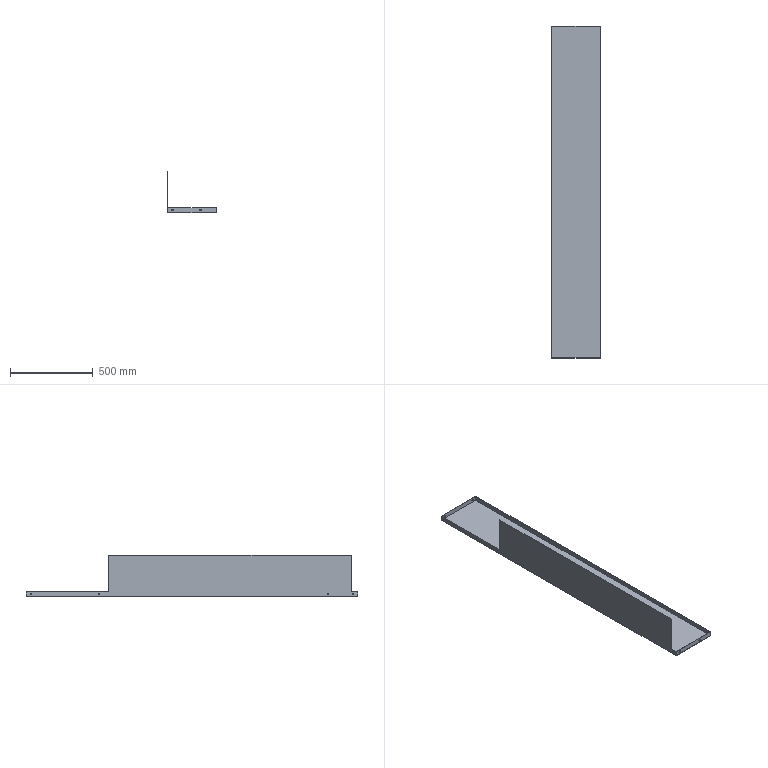Part | SolidWorks | features ICE 7, Extrusion 1, Shell 1 | 1 solid | 46 faces | box 295 x 2005 x 250 mm | volume 2083546 mm3 | cylinder 32 | plane 14 | commonest cylinder face diameters 9 x32
STEP:
#1=CARTESIAN_POINT('',(293.,175.,11.5));
#2=VERTEX_POINT('',#1);
#3=CARTESIAN_POINT('',(293.,175.,20.5));
#4=VERTEX_POINT('',#3);
#5=CARTESIAN_POINT('',(293.,175.,16.));
#6=DIRECTION('',(-1.,0.,0.));
#7=DIRECTION('',(0.,0.,1.));
#8=AXIS2_PLACEMENT_3D('',#5,#6,#7);
#9=CIRCLE('',#8,4.5);
#10=EDGE_CURVE('',#2,#4,#9,.T.);
#11=ORIENTED_EDGE('',*,*,#10,.T.);
#12=CARTESIAN_POINT('',(295.,175.,20.5));
#13=VERTEX_POINT('',#12);
#14=CARTESIAN_POINT('',(279.,175.,20.5));
#15=DIRECTION('',(1.,0.,0.));
#16=VECTOR('',#15,1000.);
#17=LINE('',#14,#16);
#18=EDGE_CURVE('',#4,#13,#17,.T.);
#19=ORIENTED_EDGE('',*,*,#18,.T.);
#20=CARTESIAN_POINT('',(295.,175.,11.5));
#21=VERTEX_POINT('',#20);
#22=CARTESIAN_POINT('',(295.,175.,16.));
#23=DIRECTION('',(1.,0.,0.));
#24=DIRECTION('',(0.,0.,-1.));
#25=AXIS2_PLACEMENT_3D('',#22,#23,#24);
#26=CIRCLE('',#25,4.5);
#27=EDGE_CURVE('',#13,#21,#26,.T.);
#28=ORIENTED_EDGE('',*,*,#27,.T.);
#29=CARTESIAN_POINT('',(279.,175.,11.5));
#30=DIRECTION('',(1.,0.,0.));
#31=VECTOR('',#30,1000.);
#32=LINE('',#29,#31);
#33=EDGE_CURVE('',#2,#21,#32,.T.);
#34=ORIENTED_EDGE('',*,*,#33,.F.);
#35=EDGE_LOOP('',(#11,#19,#28,#34));
#36=FACE_OUTER_BOUND('',#35,.T.);
#37=CARTESIAN_POINT('',(279.,175.,16.));
#38=DIRECTION('',(1.,0.,0.));
#39=DIRECTION('',(0.,0.,-1.));
#40=AXIS2_PLACEMENT_3D('',#37,#38,#39);
#41=CYLINDRICAL_SURFACE('',#40,4.5);
#42=ADVANCED_FACE('',(#36),#41,.F.);
#43=CARTESIAN_POINT('',(293.,30.,11.5));
#44=VERTEX_POINT('',#43);
#45=CARTESIAN_POINT('',(293.,30.,20.5));
#46=VERTEX_POINT('',#45);
#47=CARTESIAN_POINT('',(293.,30.,16.));
#48=DIRECTION('',(-1.,0.,0.));
#49=DIRECTION('',(0.,0.,1.));
#50=AXIS2_PLACEMENT_3D('',#47,#48,#49);
#51=CIRCLE('',#50,4.5);
#52=EDGE_CURVE('',#44,#46,#51,.T.);
#53=ORIENTED_EDGE('',*,*,#52,.T.);
#54=CARTESIAN_POINT('',(295.,30.,20.5));
#55=VERTEX_POINT('',#54);
#56=CARTESIAN_POINT('',(279.,30.,20.5));
#57=DIRECTION('',(1.,0.,0.));
#58=VECTOR('',#57,1000.);
#59=LINE('',#56,#58);
#60=EDGE_CURVE('',#46,#55,#59,.T.);
#61=ORIENTED_EDGE('',*,*,#60,.T.);
#62=CARTESIAN_POINT('',(295.,30.,11.5));
#63=VERTEX_POINT('',#62);
#64=CARTESIAN_POINT('',(295.,30.,16.));
#65=DIRECTION('',(1.,0.,0.));
#66=DIRECTION('',(0.,0.,-1.));
#67=AXIS2_PLACEMENT_3D('',#64,#65,#66);
#68=CIRCLE('',#67,4.5);
#69=EDGE_CURVE('',#55,#63,#68,.T.);
#70=ORIENTED_EDGE('',*,*,#69,.T.);
#71=CARTESIAN_POINT('',(279.,30.,11.5));
#72=DIRECTION('',(1.,0.,0.));
#73=VECTOR('',#72,1000.);
#74=LINE('',#71,#73);
#75=EDGE_CURVE('',#44,#63,#74,.T.);
#76=ORIENTED_EDGE('',*,*,#75,.F.);
#77=EDGE_LOOP('',(#53,#61,#70,#76));
#78=FACE_OUTER_BOUND('',#77,.T.);
#79=CARTESIAN_POINT('',(279.,30.,16.));
#80=DIRECTION('',(1.,0.,0.));
#81=DIRECTION('',(0.,0.,-1.));
#82=AXIS2_PLACEMENT_3D('',#79,#80,#81);
#83=CYLINDRICAL_SURFACE('',#82,4.5);
#84=ADVANCED_FACE('',(#78),#83,.F.);
#85=CARTESIAN_POINT('',(295.,235.,11.5));
#86=VERTEX_POINT('',#85);
#87=CARTESIAN_POINT('',(295.,235.,20.5));
#88=VERTEX_POINT('',#87);
#89=CARTESIAN_POINT('',(295.,235.,16.));
#90=DIRECTION('',(-1.,0.,0.));
#91=DIRECTION('',(0.,0.,1.));
#92=AXIS2_PLACEMENT_3D('',#89,#90,#91);
#93=CIRCLE('',#92,4.5);
#94=EDGE_CURVE('',#86,#88,#93,.T.);
#95=ORIENTED_EDGE('',*,*,#94,.F.);
#96=CARTESIAN_POINT('',(293.,235.,11.5));
#97=VERTEX_POINT('',#96);
#98=CARTESIAN_POINT('',(303.,235.,11.5));
#99=DIRECTION('',(-1.,0.,0.));
#100=VECTOR('',#99,1000.);
#101=LINE('',#98,#100);
#102=EDGE_CURVE('',#86,#97,#101,.T.);
#103=ORIENTED_EDGE('',*,*,#102,.T.);
#104=CARTESIAN_POINT('',(293.,235.,20.5));
#105=VERTEX_POINT('',#104);
#106=CARTESIAN_POINT('',(293.,235.,16.));
#107=DIRECTION('',(-1.,0.,0.));
#108=DIRECTION('',(0.,0.,1.));
#109=AXIS2_PLACEMENT_3D('',#106,#107,#108);
#110=CIRCLE('',#109,4.5);
#111=EDGE_CURVE('',#97,#105,#110,.T.);
#112=ORIENTED_EDGE('',*,*,#111,.T.);
#113=CARTESIAN_POINT('',(303.,235.,20.5));
#114=DIRECTION('',(-1.,0.,0.));
#115=VECTOR('',#114,1000.);
#116=LINE('',#113,#115);
#117=EDGE_CURVE('',#88,#105,#116,.T.);
#118=ORIENTED_EDGE('',*,*,#117,.F.);
#119=EDGE_LOOP('',(#95,#103,#112,#118));
#120=FACE_OUTER_BOUND('',#119,.T.);
#121=CARTESIAN_POINT('',(303.,235.,16.));
#122=DIRECTION('',(-1.,0.,0.));
#123=DIRECTION('',(0.,0.,1.));
#124=AXIS2_PLACEMENT_3D('',#121,#122,#123);
#125=CYLINDRICAL_SURFACE('',#124,4.5);
#126=ADVANCED_FACE('',(#120),#125,.F.);
#127=CARTESIAN_POINT('',(295.,776.,11.5));
#128=VERTEX_POINT('',#127);
#129=CARTESIAN_POINT('',(295.,776.,20.5));
#130=VERTEX_POINT('',#129);
#131=CARTESIAN_POINT('',(295.,776.,16.));
#132=DIRECTION('',(-1.,0.,0.));
#133=DIRECTION('',(0.,0.,1.));
#134=AXIS2_PLACEMENT_3D('',#131,#132,#133);
#135=CIRCLE('',#134,4.5);
#136=EDGE_CURVE('',#128,#130,#135,.T.);
#137=ORIENTED_EDGE('',*,*,#136,.F.);
#138=CARTESIAN_POINT('',(293.,776.,11.5));
#139=VERTEX_POINT('',#138);
#140=CARTESIAN_POINT('',(303.,776.,11.5));
#141=DIRECTION('',(-1.,0.,0.));
#142=VECTOR('',#141,1000.);
#143=LINE('',#140,#142);
#144=EDGE_CURVE('',#128,#139,#143,.T.);
#145=ORIENTED_EDGE('',*,*,#144,.T.);
#146=CARTESIAN_POINT('',(293.,776.,20.5));
#147=VERTEX_POINT('',#146);
#148=CARTESIAN_POINT('',(293.,776.,16.));
#149=DIRECTION('',(-1.,0.,0.));
#150=DIRECTION('',(0.,0.,1.));
#151=AXIS2_PLACEMENT_3D('',#148,#149,#150);
#152=CIRCLE('',#151,4.5);
#153=EDGE_CURVE('',#139,#147,#152,.T.);
#154=ORIENTED_EDGE('',*,*,#153,.T.);
#155=CARTESIAN_POINT('',(303.,776.,20.5));
#156=DIRECTION('',(-1.,0.,0.));
#157=VECTOR('',#156,1000.);
#158=LINE('',#155,#157);
#159=EDGE_CURVE('',#130,#147,#158,.T.);
#160=ORIENTED_EDGE('',*,*,#159,.F.);
#161=EDGE_LOOP('',(#137,#145,#154,#160));
#162=FACE_OUTER_BOUND('',#161,.T.);
#163=CARTESIAN_POINT('',(303.,776.,16.));
#164=DIRECTION('',(-1.,0.,0.));
#165=DIRECTION('',(0.,0.,1.));
#166=AXIS2_PLACEMENT_3D('',#163,#164,#165);
#167=CYLINDRICAL_SURFACE('',#166,4.5);
#168=ADVANCED_FACE('',(#162),#167,.F.);
#169=CARTESIAN_POINT('',(295.,1317.,11.5));
#170=VERTEX_POINT('',#169);
#171=CARTESIAN_POINT('',(295.,1317.,20.5));
#172=VERTEX_POINT('',#171);
#173=CARTESIAN_POINT('',(295.,1317.,16.));
#174=DIRECTION('',(-1.,0.,0.));
#175=DIRECTION('',(0.,0.,1.));
#176=AXIS2_PLACEMENT_3D('',#173,#174,#175);
#177=CIRCLE('',#176,4.5);
#178=EDGE_CURVE('',#170,#172,#177,.T.);
#179=ORIENTED_EDGE('',*,*,#178,.F.);
#180=CARTESIAN_POINT('',(293.,1317.,11.5));
#181=VERTEX_POINT('',#180);
#182=CARTESIAN_POINT('',(303.,1317.,11.5));
#183=DIRECTION('',(-1.,0.,0.));
#184=VECTOR('',#183,1000.);
#185=LINE('',#182,#184);
#186=EDGE_CURVE('',#170,#181,#185,.T.);
#187=ORIENTED_EDGE('',*,*,#186,.T.);
#188=CARTESIAN_POINT('',(293.,1317.,20.5));
#189=VERTEX_POINT('',#188);
#190=CARTESIAN_POINT('',(293.,1317.,16.));
#191=DIRECTION('',(-1.,0.,0.));
#192=DIRECTION('',(0.,0.,1.));
#193=AXIS2_PLACEMENT_3D('',#190,#191,#192);
#194=CIRCLE('',#193,4.5);
#195=EDGE_CURVE('',#181,#189,#194,.T.);
#196=ORIENTED_EDGE('',*,*,#195,.T.);
#197=CARTESIAN_POINT('',(303.,1317.,20.5));
#198=DIRECTION('',(-1.,0.,0.));
#199=VECTOR('',#198,1000.);
#200=LINE('',#197,#199);
#201=EDGE_CURVE('',#172,#189,#200,.T.);
#202=ORIENTED_EDGE('',*,*,#201,.F.);
#203=EDGE_LOOP('',(#179,#187,#196,#202));
#204=FACE_OUTER_BOUND('',#203,.T.);
#205=CARTESIAN_POINT('',(303.,1317.,16.));
#206=DIRECTION('',(-1.,0.,0.));
#207=DIRECTION('',(0.,0.,1.));
#208=AXIS2_PLACEMENT_3D('',#205,#206,#207);
#209=CYLINDRICAL_SURFACE('',#208,4.5);
#210=ADVANCED_FACE('',(#204),#209,.F.);
#211=CARTESIAN_POINT('',(295.,1377.,11.5));
#212=VERTEX_POINT('',#211);
#213=CARTESIAN_POINT('',(295.,1377.,20.5));
#214=VERTEX_POINT('',#213);
#215=CARTESIAN_POINT('',(295.,1377.,16.));
#216=DIRECTION('',(-1.,0.,0.));
#217=DIRECTION('',(0.,0.,1.));
#218=AXIS2_PLACEMENT_3D('',#215,#216,#217);
#219=CIRCLE('',#218,4.5);
#220=EDGE_CURVE('',#212,#214,#219,.T.);
#221=ORIENTED_EDGE('',*,*,#220,.F.);
#222=CARTESIAN_POINT('',(293.,1377.,11.5));
#223=VERTEX_POINT('',#222);
#224=CARTESIAN_POINT('',(303.,1377.,11.5));
#225=DIRECTION('',(-1.,0.,0.));
#226=VECTOR('',#225,1000.);
#227=LINE('',#224,#226);
#228=EDGE_CURVE('',#212,#223,#227,.T.);
#229=ORIENTED_EDGE('',*,*,#228,.T.);
#230=CARTESIAN_POINT('',(293.,1377.,20.5));
#231=VERTEX_POINT('',#230);
#232=CARTESIAN_POINT('',(293.,1377.,16.));
#233=DIRECTION('',(-1.,0.,0.));
#234=DIRECTION('',(0.,0.,1.));
#235=AXIS2_PLACEMENT_3D('',#232,#233,#234);
#236=CIRCLE('',#235,4.5);
#237=EDGE_CURVE('',#223,#231,#236,.T.);
#238=ORIENTED_EDGE('',*,*,#237,.T.);
#239=CARTESIAN_POINT('',(303.,1377.,20.5));
#240=DIRECTION('',(-1.,0.,0.));
#241=VECTOR('',#240,1000.);
#242=LINE('',#239,#241);
#243=EDGE_CURVE('',#214,#231,#242,.T.);
#244=ORIENTED_EDGE('',*,*,#243,.F.);
#245=EDGE_LOOP('',(#221,#229,#238,#244));
#246=FACE_OUTER_BOUND('',#245,.T.);
#247=CARTESIAN_POINT('',(303.,1377.,16.));
#248=DIRECTION('',(-1.,0.,0.));
#249=DIRECTION('',(0.,0.,1.));
#250=AXIS2_PLACEMENT_3D('',#247,#248,#249);
#251=CYLINDRICAL_SURFACE('',#250,4.5);
#252=ADVANCED_FACE('',(#246),#251,.F.);
#253=CARTESIAN_POINT('',(295.,1676.,11.5));
#254=VERTEX_POINT('',#253);
#255=CARTESIAN_POINT('',(295.,1676.,20.5));
#256=VERTEX_POINT('',#255);
#257=CARTESIAN_POINT('',(295.,1676.,16.));
#258=DIRECTION('',(-1.,0.,0.));
#259=DIRECTION('',(0.,0.,1.));
#260=AXIS2_PLACEMENT_3D('',#257,#258,#259);
#261=CIRCLE('',#260,4.5);
#262=EDGE_CURVE('',#254,#256,#261,.T.);
#263=ORIENTED_EDGE('',*,*,#262,.F.);
#264=CARTESIAN_POINT('',(293.,1676.,11.5));
#265=VERTEX_POINT('',#264);
#266=CARTESIAN_POINT('',(303.,1676.,11.5));
#267=DIRECTION('',(-1.,0.,0.));
#268=VECTOR('',#267,1000.);
#269=LINE('',#266,#268);
#270=EDGE_CURVE('',#254,#265,#269,.T.);
#271=ORIENTED_EDGE('',*,*,#270,.T.);
#272=CARTESIAN_POINT('',(293.,1676.,20.5));
#273=VERTEX_POINT('',#272);
#274=CARTESIAN_POINT('',(293.,1676.,16.));
#275=DIRECTION('',(-1.,0.,0.));
#276=DIRECTION('',(0.,0.,1.));
#277=AXIS2_PLACEMENT_3D('',#274,#275,#276);
#278=CIRCLE('',#277,4.5);
#279=EDGE_CURVE('',#265,#273,#278,.T.);
#280=ORIENTED_EDGE('',*,*,#279,.T.);
#281=CARTESIAN_POINT('',(303.,1676.,20.5));
#282=DIRECTION('',(-1.,0.,0.));
#283=VECTOR('',#282,1000.);
#284=LINE('',#281,#283);
#285=EDGE_CURVE('',#256,#273,#284,.T.);
#286=ORIENTED_EDGE('',*,*,#285,.F.);
#287=EDGE_LOOP('',(#263,#271,#280,#286));
#288=FACE_OUTER_BOUND('',#287,.T.);
#289=CARTESIAN_POINT('',(303.,1676.,16.));
#290=DIRECTION('',(-1.,0.,0.));
#291=DIRECTION('',(0.,0.,1.));
#292=AXIS2_PLACEMENT_3D('',#289,#290,#291);
#293=CYLINDRICAL_SURFACE('',#292,4.5);
#294=ADVANCED_FACE('',(#288),#293,.F.);
#295=CARTESIAN_POINT('',(295.,1975.,11.5));
#296=VERTEX_POINT('',#295);
#297=CARTESIAN_POINT('',(295.,1975.,20.5));
#298=VERTEX_POINT('',#297);
#299=CARTESIAN_POINT('',(295.,1975.,16.));
#300=DIRECTION('',(-1.,0.,0.));
#301=DIRECTION('',(0.,0.,1.));
#302=AXIS2_PLACEMENT_3D('',#299,#300,#301);
#303=CIRCLE('',#302,4.5);
#304=EDGE_CURVE('',#296,#298,#303,.T.);
#305=ORIENTED_EDGE('',*,*,#304,.F.);
#306=CARTESIAN_POINT('',(293.,1975.,11.5));
#307=VERTEX_POINT('',#306);
#308=CARTESIAN_POINT('',(303.,1975.,11.5));
#309=DIRECTION('',(-1.,0.,0.));
#310=VECTOR('',#309,1000.);
#311=LINE('',#308,#310);
#312=EDGE_CURVE('',#296,#307,#311,.T.);
#313=ORIENTED_EDGE('',*,*,#312,.T.);
#314=CARTESIAN_POINT('',(293.,1975.,20.5));
#315=VERTEX_POINT('',#314);
#316=CARTESIAN_POINT('',(293.,1975.,16.));
#317=DIRECTION('',(-1.,0.,0.));
#318=DIRECTION('',(0.,0.,1.));
#319=AXIS2_PLACEMENT_3D('',#316,#317,#318);
#320=CIRCLE('',#319,4.5);
#321=EDGE_CURVE('',#307,#315,#320,.T.);
#322=ORIENTED_EDGE('',*,*,#321,.T.);
#323=CARTESIAN_POINT('',(303.,1975.,20.5));
#324=DIRECTION('',(-1.,0.,0.));
#325=VECTOR('',#324,1000.);
#326=LINE('',#323,#325);
#327=EDGE_CURVE('',#298,#315,#326,.T.);
#328=ORIENTED_EDGE('',*,*,#327,.F.);
#329=EDGE_LOOP('',(#305,#313,#322,#328));
#330=FACE_OUTER_BOUND('',#329,.T.);
#331=CARTESIAN_POINT('',(303.,1975.,16.));
#332=DIRECTION('',(-1.,0.,0.));
#333=DIRECTION('',(0.,0.,1.));
#334=AXIS2_PLACEMENT_3D('',#331,#332,#333);
#335=CYLINDRICAL_SURFACE('',#334,4.5);
#336=ADVANCED_FACE('',(#330),#335,.F.);
#337=CARTESIAN_POINT('',(265.,2003.,20.5));
#338=VERTEX_POINT('',#337);
#339=CARTESIAN_POINT('',(265.,2003.,11.5));
#340=VERTEX_POINT('',#339);
#341=CARTESIAN_POINT('',(265.,2003.,16.));
#342=DIRECTION('',(0.,-1.,0.));
#343=DIRECTION('',(0.,0.,-1.));
#344=AXIS2_PLACEMENT_3D('',#341,#342,#343);
#345=CIRCLE('',#344,4.5);
#346=EDGE_CURVE('',#338,#340,#345,.T.);
#347=ORIENTED_EDGE('',*,*,#346,.T.);
#348=CARTESIAN_POINT('',(265.,2005.,11.5));
#349=VERTEX_POINT('',#348);
#350=CARTESIAN_POINT('',(265.,1995.,11.5));
#351=DIRECTION('',(0.,1.,0.));
#352=VECTOR('',#351,1000.);
#353=LINE('',#350,#352);
#354=EDGE_CURVE('',#340,#349,#353,.T.);
#355=ORIENTED_EDGE('',*,*,#354,.T.);
#356=CARTESIAN_POINT('',(265.,2005.,20.5));
#357=VERTEX_POINT('',#356);
#358=CARTESIAN_POINT('',(265.,2005.,16.));
#359=DIRECTION('',(0.,1.,0.));
#360=DIRECTION('',(0.,0.,1.));
#361=AXIS2_PLACEMENT_3D('',#358,#359,#360);
#362=CIRCLE('',#361,4.5);
#363=EDGE_CURVE('',#349,#357,#362,.T.);
#364=ORIENTED_EDGE('',*,*,#363,.T.);
#365=CARTESIAN_POINT('',(265.,1995.,20.5));
#366=DIRECTION('',(0.,1.,0.));
#367=VECTOR('',#366,1000.);
#368=LINE('',#365,#367);
#369=EDGE_CURVE('',#338,#357,#368,.T.);
#370=ORIENTED_EDGE('',*,*,#369,.F.);
#371=EDGE_LOOP('',(#347,#355,#364,#370));
#372=FACE_OUTER_BOUND('',#371,.T.);
#373=CARTESIAN_POINT('',(265.,1995.,16.));
#374=DIRECTION('',(0.,1.,0.));
#375=DIRECTION('',(0.,0.,1.));
#376=AXIS2_PLACEMENT_3D('',#373,#374,#375);
#377=CYLINDRICAL_SURFACE('',#376,4.5);
#378=ADVANCED_FACE('',(#372),#377,.F.);
#379=CARTESIAN_POINT('',(30.,2003.,20.5));
#380=VERTEX_POINT('',#379);
#381=CARTESIAN_POINT('',(30.,2003.,11.5));
#382=VERTEX_POINT('',#381);
#383=CARTESIAN_POINT('',(30.,2003.,16.));
#384=DIRECTION('',(0.,-1.,0.));
#385=DIRECTION('',(0.,0.,-1.));
#386=AXIS2_PLACEMENT_3D('',#383,#384,#385);
#387=CIRCLE('',#386,4.5);
#388=EDGE_CURVE('',#380,#382,#387,.T.);
#389=ORIENTED_EDGE('',*,*,#388,.T.);
#390=CARTESIAN_POINT('',(30.,2005.,11.5));
#391=VERTEX_POINT('',#390);
#392=CARTESIAN_POINT('',(30.,1995.,11.5));
#393=DIRECTION('',(0.,1.,0.));
#394=VECTOR('',#393,1000.);
#395=LINE('',#392,#394);
#396=EDGE_CURVE('',#382,#391,#395,.T.);
#397=ORIENTED_EDGE('',*,*,#396,.T.);
#398=CARTESIAN_POINT('',(30.,2005.,20.5));
#399=VERTEX_POINT('',#398);
#400=CARTESIAN_POINT('',(30.,2005.,16.));
#401=DIRECTION('',(0.,1.,0.));
#402=DIRECTION('',(0.,0.,1.));
#403=AXIS2_PLACEMENT_3D('',#400,#401,#402);
#404=CIRCLE('',#403,4.5);
#405=EDGE_CURVE('',#391,#399,#404,.T.);
#406=ORIENTED_EDGE('',*,*,#405,.T.);
#407=CARTESIAN_POINT('',(30.,1995.,20.5));
#408=DIRECTION('',(0.,1.,0.));
#409=VECTOR('',#408,1000.);
#410=LINE('',#407,#409);
#411=EDGE_CURVE('',#380,#399,#410,.T.);
#412=ORIENTED_EDGE('',*,*,#411,.F.);
#413=EDGE_LOOP('',(#389,#397,#406,#412));
#414=FACE_OUTER_BOUND('',#413,.T.);
#415=CARTESIAN_POINT('',(30.,1995.,16.));
#416=DIRECTION('',(0.,1.,0.));
#417=DIRECTION('',(0.,0.,1.));
#418=AXIS2_PLACEMENT_3D('',#415,#416,#417);
#419=CYLINDRICAL_SURFACE('',#418,4.5);
#420=ADVANCED_FACE('',(#414),#419,.F.);
#421=CARTESIAN_POINT('',(0.,1563.,20.5));
#422=VERTEX_POINT('',#421);
#423=CARTESIAN_POINT('',(0.,1563.,11.5));
#424=VERTEX_POINT('',#423);
#425=CARTESIAN_POINT('',(0.,1563.,16.));
#426=DIRECTION('',(1.,0.,0.));
#427=DIRECTION('',(0.,0.,-1.));
#428=AXIS2_PLACEMENT_3D('',#425,#426,#427);
#429=CIRCLE('',#428,4.5);
#430=EDGE_CURVE('',#422,#424,#429,.T.);
#431=ORIENTED_EDGE('',*,*,#430,.F.);
#432=CARTESIAN_POINT('',(2.,1563.,20.5));
#433=VERTEX_POINT('',#432);
#434=CARTESIAN_POINT('',(-70.,1563.,20.5));
#435=DIRECTION('',(1.,0.,0.));
#436=VECTOR('',#435,1000.);
#437=LINE('',#434,#436);
#438=EDGE_CURVE('',#422,#433,#437,.T.);
#439=ORIENTED_EDGE('',*,*,#438,.T.);
#440=CARTESIAN_POINT('',(2.,1563.,11.5));
#441=VERTEX_POINT('',#440);
#442=CARTESIAN_POINT('',(2.,1563.,16.));
#443=DIRECTION('',(1.,0.,0.));
#444=DIRECTION('',(0.,0.,-1.));
#445=AXIS2_PLACEMENT_3D('',#442,#443,#444);
#446=CIRCLE('',#445,4.5);
#447=EDGE_CURVE('',#433,#441,#446,.T.);
#448=ORIENTED_EDGE('',*,*,#447,.T.);
#449=CARTESIAN_POINT('',(-70.,1563.,11.5));
#450=DIRECTION('',(1.,0.,0.));
#451=VECTOR('',#450,1000.);
#452=LINE('',#449,#451);
#453=EDGE_CURVE('',#424,#441,#452,.T.);
#454=ORIENTED_EDGE('',*,*,#453,.F.);
#455=EDGE_LOOP('',(#431,#439,#448,#454));
#456=FACE_OUTER_BOUND('',#455,.T.);
#457=CARTESIAN_POINT('',(-70.,1563.,16.));
#458=DIRECTION('',(1.,0.,0.));
#459=DIRECTION('',(0.,0.,-1.));
#460=AXIS2_PLACEMENT_3D('',#457,#458,#459);
#461=CYLINDRICAL_SURFACE('',#460,4.5);
#462=ADVANCED_FACE('',(#456),#461,.F.);
#463=CARTESIAN_POINT('',(0.,1975.,20.5));
#464=VERTEX_POINT('',#463);
#465=CARTESIAN_POINT('',(0.,1975.,11.5));
#466=VERTEX_POINT('',#465);
#467=CARTESIAN_POINT('',(0.,1975.,16.));
#468=DIRECTION('',(1.,0.,0.));
#469=DIRECTION('',(0.,0.,-1.));
#470=AXIS2_PLACEMENT_3D('',#467,#468,#469);
#471=CIRCLE('',#470,4.5);
#472=EDGE_CURVE('',#464,#466,#471,.T.);
#473=ORIENTED_EDGE('',*,*,#472,.F.);
#474=CARTESIAN_POINT('',(2.,1975.,20.5));
#475=VERTEX_POINT('',#474);
#476=CARTESIAN_POINT('',(-70.,1975.,20.5));
#477=DIRECTION('',(1.,0.,0.));
#478=VECTOR('',#477,1000.);
#479=LINE('',#476,#478);
#480=EDGE_CURVE('',#464,#475,#479,.T.);
#481=ORIENTED_EDGE('',*,*,#480,.T.);
#482=CARTESIAN_POINT('',(2.,1975.,11.5));
#483=VERTEX_POINT('',#482);
#484=CARTESIAN_POINT('',(2.,1975.,16.));
#485=DIRECTION('',(1.,0.,0.));
#486=DIRECTION('',(0.,0.,-1.));
#487=AXIS2_PLACEMENT_3D('',#484,#485,#486);
#488=CIRCLE('',#487,4.5);
#489=EDGE_CURVE('',#475,#483,#488,.T.);
#490=ORIENTED_EDGE('',*,*,#489,.T.);
#491=CARTESIAN_POINT('',(-70.,1975.,11.5));
#492=DIRECTION('',(1.,0.,0.));
#493=VECTOR('',#492,1000.);
#494=LINE('',#491,#493);
#495=EDGE_CURVE('',#466,#483,#494,.T.);
#496=ORIENTED_EDGE('',*,*,#495,.F.);
#497=EDGE_LOOP('',(#473,#481,#490,#496));
#498=FACE_OUTER_BOUND('',#497,.T.);
#499=CARTESIAN_POINT('',(-70.,1975.,16.));
#500=DIRECTION('',(1.,0.,0.));
#501=DIRECTION('',(0.,0.,-1.));
#502=AXIS2_PLACEMENT_3D('',#499,#500,#501);
#503=CYLINDRICAL_SURFACE('',#502,4.5);
#504=ADVANCED_FACE('',(#498),#503,.F.);
#505=CARTESIAN_POINT('',(0.,180.,20.5));
#506=VERTEX_POINT('',#505);
#507=CARTESIAN_POINT('',(0.,180.,11.5));
#508=VERTEX_POINT('',#507);
#509=CARTESIAN_POINT('',(0.,180.,16.));
#510=DIRECTION('',(1.,0.,0.));
#511=DIRECTION('',(0.,0.,-1.));
#512=AXIS2_PLACEMENT_3D('',#509,#510,#511);
#513=CIRCLE('',#512,4.5);
#514=EDGE_CURVE('',#506,#508,#513,.T.);
#515=ORIENTED_EDGE('',*,*,#514,.F.);
#516=CARTESIAN_POINT('',(2.,180.,20.5));
#517=VERTEX_POINT('',#516);
#518=CARTESIAN_POINT('',(-114.,180.,20.5));
#519=DIRECTION('',(1.,0.,0.));
#520=VECTOR('',#519,1000.);
#521=LINE('',#518,#520);
#522=EDGE_CURVE('',#506,#517,#521,.T.);
#523=ORIENTED_EDGE('',*,*,#522,.T.);
#524=CARTESIAN_POINT('',(2.,180.,11.5));
#525=VERTEX_POINT('',#524);
#526=CARTESIAN_POINT('',(2.,180.,16.));
#527=DIRECTION('',(1.,0.,0.));
#528=DIRECTION('',(0.,0.,-1.));
#529=AXIS2_PLACEMENT_3D('',#526,#527,#528);
#530=CIRCLE('',#529,4.5);
#531=EDGE_CURVE('',#517,#525,#530,.T.);
#532=ORIENTED_EDGE('',*,*,#531,.T.);
#533=CARTESIAN_POINT('',(-114.,180.,11.5));
#534=DIRECTION('',(1.,0.,0.));
#535=VECTOR('',#534,1000.);
#536=LINE('',#533,#535);
#537=EDGE_CURVE('',#508,#525,#536,.T.);
#538=ORIENTED_EDGE('',*,*,#537,.F.);
#539=EDGE_LOOP('',(#515,#523,#532,#538));
#540=FACE_OUTER_BOUND('',#539,.T.);
#541=CARTESIAN_POINT('',(-114.,180.,16.));
#542=DIRECTION('',(1.,0.,0.));
#543=DIRECTION('',(0.,0.,-1.));
#544=AXIS2_PLACEMENT_3D('',#541,#542,#543);
#545=CYLINDRICAL_SURFACE('',#544,4.5);
#546=ADVANCED_FACE('',(#540),#545,.F.);
#547=CARTESIAN_POINT('',(0.,30.,20.5));
#548=VERTEX_POINT('',#547);
#549=CARTESIAN_POINT('',(0.,30.,11.5));
#550=VERTEX_POINT('',#549);
#551=CARTESIAN_POINT('',(0.,30.,16.));
#552=DIRECTION('',(1.,0.,0.));
#553=DIRECTION('',(0.,0.,-1.));
#554=AXIS2_PLACEMENT_3D('',#551,#552,#553);
#555=CIRCLE('',#554,4.5);
#556=EDGE_CURVE('',#548,#550,#555,.T.);
#557=ORIENTED_EDGE('',*,*,#556,.F.);
#558=CARTESIAN_POINT('',(2.,30.,20.5));
#559=VERTEX_POINT('',#558);
#560=CARTESIAN_POINT('',(-114.,30.,20.5));
#561=DIRECTION('',(1.,0.,0.));
#562=VECTOR('',#561,1000.);
#563=LINE('',#560,#562);
#564=EDGE_CURVE('',#548,#559,#563,.T.);
#565=ORIENTED_EDGE('',*,*,#564,.T.);
#566=CARTESIAN_POINT('',(2.,30.,11.5));
#567=VERTEX_POINT('',#566);
#568=CARTESIAN_POINT('',(2.,30.,16.));
#569=DIRECTION('',(1.,0.,0.));
#570=DIRECTION('',(0.,0.,-1.));
#571=AXIS2_PLACEMENT_3D('',#568,#569,#570);
#572=CIRCLE('',#571,4.5);
#573=EDGE_CURVE('',#559,#567,#572,.T.);
#574=ORIENTED_EDGE('',*,*,#573,.T.);
#575=CARTESIAN_POINT('',(-114.,30.,11.5));
#576=DIRECTION('',(1.,0.,0.));
#577=VECTOR('',#576,1000.);
#578=LINE('',#575,#577);
#579=EDGE_CURVE('',#550,#567,#578,.T.);
#580=ORIENTED_EDGE('',*,*,#579,.F.);
#581=EDGE_LOOP('',(#557,#565,#574,#580));
#582=FACE_OUTER_BOUND('',#581,.T.);
#583=CARTESIAN_POINT('',(-114.,30.,16.));
#584=DIRECTION('',(1.,0.,0.));
#585=DIRECTION('',(0.,0.,-1.));
#586=AXIS2_PLACEMENT_3D('',#583,#584,#585);
#587=CYLINDRICAL_SURFACE('',#586,4.5);
#588=ADVANCED_FACE('',(#582),#587,.F.);
#589=CARTESIAN_POINT('',(200.,0.,11.5));
#590=VERTEX_POINT('',#589);
#591=CARTESIAN_POINT('',(200.,0.,20.5));
#592=VERTEX_POINT('',#591);
#593=CARTESIAN_POINT('',(200.,0.,16.));
#594=DIRECTION('',(0.,1.,0.));
#595=DIRECTION('',(0.,0.,1.));
#596=AXIS2_PLACEMENT_3D('',#593,#594,#595);
#597=CIRCLE('',#596,4.5);
#598=EDGE_CURVE('',#590,#592,#597,.T.);
#599=ORIENTED_EDGE('',*,*,#598,.F.);
#600=CARTESIAN_POINT('',(200.,2.,11.5));
#601=VERTEX_POINT('',#600);
#602=CARTESIAN_POINT('',(200.,-8.,11.5));
#603=DIRECTION('',(0.,1.,0.));
#604=VECTOR('',#603,1000.);
#605=LINE('',#602,#604);
#606=EDGE_CURVE('',#590,#601,#605,.T.);
#607=ORIENTED_EDGE('',*,*,#606,.T.);
#608=CARTESIAN_POINT('',(200.,2.,20.5));
#609=VERTEX_POINT('',#608);
#610=CARTESIAN_POINT('',(200.,2.,16.));
#611=DIRECTION('',(0.,1.,0.));
#612=DIRECTION('',(0.,0.,1.));
#613=AXIS2_PLACEMENT_3D('',#610,#611,#612);
#614=CIRCLE('',#613,4.5);
#615=EDGE_CURVE('',#601,#609,#614,.T.);
#616=ORIENTED_EDGE('',*,*,#615,.T.);
#617=CARTESIAN_POINT('',(200.,-8.,20.5));
#618=DIRECTION('',(0.,1.,0.));
#619=VECTOR('',#618,1000.);
#620=LINE('',#617,#619);
#621=EDGE_CURVE('',#592,#609,#620,.T.);
#622=ORIENTED_EDGE('',*,*,#621,.F.);
#623=EDGE_LOOP('',(#599,#607,#616,#622));
#624=FACE_OUTER_BOUND('',#623,.T.);
#625=CARTESIAN_POINT('',(200.,-8.,16.));
#626=DIRECTION('',(0.,1.,0.));
#627=DIRECTION('',(0.,0.,1.));
#628=AXIS2_PLACEMENT_3D('',#625,#626,#627);
#629=CYLINDRICAL_SURFACE('',#628,4.5);
#630=ADVANCED_FACE('',(#624),#629,.F.);
#631=CARTESIAN_POINT('',(30.,0.,11.5));
#632=VERTEX_POINT('',#631);
#633=CARTESIAN_POINT('',(30.,0.,20.5));
#634=VERTEX_POINT('',#633);
#635=CARTESIAN_POINT('',(30.,0.,16.));
#636=DIRECTION('',(0.,1.,0.));
#637=DIRECTION('',(0.,0.,1.));
#638=AXIS2_PLACEMENT_3D('',#635,#636,#637);
#639=CIRCLE('',#638,4.5);
#640=EDGE_CURVE('',#632,#634,#639,.T.);
#641=ORIENTED_EDGE('',*,*,#640,.F.);
#642=CARTESIAN_POINT('',(30.,2.,11.5));
#643=VERTEX_POINT('',#642);
#644=CARTESIAN_POINT('',(30.,-8.,11.5));
#645=DIRECTION('',(0.,1.,0.));
#646=VECTOR('',#645,1000.);
#647=LINE('',#644,#646);
#648=EDGE_CURVE('',#632,#643,#647,.T.);
#649=ORIENTED_EDGE('',*,*,#648,.T.);
#650=CARTESIAN_POINT('',(30.,2.,20.5));
#651=VERTEX_POINT('',#650);
#652=CARTESIAN_POINT('',(30.,2.,16.));
#653=DIRECTION('',(0.,1.,0.));
#654=DIRECTION('',(0.,0.,1.));
#655=AXIS2_PLACEMENT_3D('',#652,#653,#654);
#656=CIRCLE('',#655,4.5);
#657=EDGE_CURVE('',#643,#651,#656,.T.);
#658=ORIENTED_EDGE('',*,*,#657,.T.);
#659=CARTESIAN_POINT('',(30.,-8.,20.5));
#660=DIRECTION('',(0.,1.,0.));
#661=VECTOR('',#660,1000.);
#662=LINE('',#659,#661);
#663=EDGE_CURVE('',#634,#651,#662,.T.);
#664=ORIENTED_EDGE('',*,*,#663,.F.);
#665=EDGE_LOOP('',(#641,#649,#658,#664));
#666=FACE_OUTER_BOUND('',#665,.T.);
#667=CARTESIAN_POINT('',(30.,-8.,16.));
#668=DIRECTION('',(0.,1.,0.));
#669=DIRECTION('',(0.,0.,1.));
#670=AXIS2_PLACEMENT_3D('',#667,#668,#669);
#671=CYLINDRICAL_SURFACE('',#670,4.5);
#672=ADVANCED_FACE('',(#666),#671,.F.);
#673=CARTESIAN_POINT('',(2.,1507.,30.));
#674=VERTEX_POINT('',#673);
#675=CARTESIAN_POINT('',(0.,1507.,30.));
#676=VERTEX_POINT('',#675);
#677=CARTESIAN_POINT('',(0.,1507.,30.));
#678=DIRECTION('',(-1.,0.,0.));
#679=VECTOR('',#678,1000.);
#680=LINE('',#677,#679);
#681=EDGE_CURVE('',#674,#676,#680,.T.);
#682=ORIENTED_EDGE('',*,*,#681,.F.);
#683=CARTESIAN_POINT('',(2.,2003.,30.));
#684=VERTEX_POINT('',#683);
#685=CARTESIAN_POINT('',(2.,2005.,30.));
#686=DIRECTION('',(0.,-1.,0.));
#687=VECTOR('',#686,1000.);
#688=LINE('',#685,#687);
#689=EDGE_CURVE('',#684,#674,#688,.T.);
#690=ORIENTED_EDGE('',*,*,#689,.F.);
#691=CARTESIAN_POINT('',(293.,2003.,30.));
#692=VERTEX_POINT('',#691);
#693=CARTESIAN_POINT('',(0.,2003.,30.));
#694=DIRECTION('',(-1.,0.,0.));
#695=VECTOR('',#694,1000.);
#696=LINE('',#693,#695);
#697=EDGE_CURVE('',#692,#684,#696,.T.);
#698=ORIENTED_EDGE('',*,*,#697,.F.);
#699=CARTESIAN_POINT('',(293.,2.,30.));
#700=VERTEX_POINT('',#699);
#701=CARTESIAN_POINT('',(293.,2005.,30.));
#702=DIRECTION('',(0.,1.,0.));
#703=VECTOR('',#702,1000.);
#704=LINE('',#701,#703);
#705=EDGE_CURVE('',#700,#692,#704,.T.);
#706=ORIENTED_EDGE('',*,*,#705,.F.);
#707=CARTESIAN_POINT('',(2.,2.,30.));
#708=VERTEX_POINT('',#707);
#709=CARTESIAN_POINT('',(0.,2.,30.));
#710=DIRECTION('',(1.,0.,0.));
#711=VECTOR('',#710,1000.);
#712=LINE('',#709,#711);
#713=EDGE_CURVE('',#708,#700,#712,.T.);
#714=ORIENTED_EDGE('',*,*,#713,.F.);
#715=CARTESIAN_POINT('',(2.,40.,30.));
#716=VERTEX_POINT('',#715);
#717=CARTESIAN_POINT('',(2.,2005.,30.));
#718=DIRECTION('',(0.,-1.,0.));
#719=VECTOR('',#718,1000.);
#720=LINE('',#717,#719);
#721=EDGE_CURVE('',#716,#708,#720,.T.);
#722=ORIENTED_EDGE('',*,*,#721,.F.);
#723=CARTESIAN_POINT('',(0.,40.,30.));
#724=VERTEX_POINT('',#723);
#725=CARTESIAN_POINT('',(0.,40.,30.));
#726=DIRECTION('',(1.,0.,0.));
#727=VECTOR('',#726,1000.);
#728=LINE('',#725,#727);
#729=EDGE_CURVE('',#724,#716,#728,.T.);
#730=ORIENTED_EDGE('',*,*,#729,.F.);
#731=CARTESIAN_POINT('',(0.,0.,30.));
#732=VERTEX_POINT('',#731);
#733=CARTESIAN_POINT('',(0.,0.,30.));
#734=DIRECTION('',(0.,-1.,0.));
#735=VECTOR('',#734,1000.);
#736=LINE('',#733,#735);
#737=EDGE_CURVE('',#724,#732,#736,.T.);
#738=ORIENTED_EDGE('',*,*,#737,.T.);
#739=CARTESIAN_POINT('',(295.,0.,30.));
#740=VERTEX_POINT('',#739);
#741=CARTESIAN_POINT('',(0.,0.,30.));
#742=DIRECTION('',(1.,0.,0.));
#743=VECTOR('',#742,1000.);
#744=LINE('',#741,#743);
#745=EDGE_CURVE('',#732,#740,#744,.T.);
#746=ORIENTED_EDGE('',*,*,#745,.T.);
#747=CARTESIAN_POINT('',(295.,2005.,30.));
#748=VERTEX_POINT('',#747);
#749=CARTESIAN_POINT('',(295.,0.,30.));
#750=DIRECTION('',(0.,1.,0.));
#751=VECTOR('',#750,1000.);
#752=LINE('',#749,#751);
#753=EDGE_CURVE('',#740,#748,#752,.T.);
#754=ORIENTED_EDGE('',*,*,#753,.T.);
#755=CARTESIAN_POINT('',(0.,2005.,30.));
#756=VERTEX_POINT('',#755);
#757=CARTESIAN_POINT('',(0.,2005.,30.));
#758=DIRECTION('',(-1.,0.,0.));
#759=VECTOR('',#758,1000.);
#760=LINE('',#757,#759);
#761=EDGE_CURVE('',#748,#756,#760,.T.);
#762=ORIENTED_EDGE('',*,*,#761,.T.);
#763=CARTESIAN_POINT('',(0.,0.,30.));
#764=DIRECTION('',(0.,-1.,0.));
#765=VECTOR('',#764,1000.);
#766=LINE('',#763,#765);
#767=EDGE_CURVE('',#756,#676,#766,.T.);
#768=ORIENTED_EDGE('',*,*,#767,.T.);
#769=EDGE_LOOP('',(#682,#690,#698,#706,#714,#722,#730,#738,#746,#754,#762,#768));
#770=FACE_OUTER_BOUND('',#769,.T.);
#771=CARTESIAN_POINT('',(0.,2005.,30.));
#772=DIRECTION('',(0.,0.,-1.));
#773=DIRECTION('',(-1.,0.,0.));
#774=AXIS2_PLACEMENT_3D('',#771,#772,#773);
#775=PLANE('',#774);
#776=ADVANCED_FACE('',(#770),#775,.F.);
#777=CARTESIAN_POINT('',(0.,1563.,16.));
#778=DIRECTION('',(1.,0.,0.));
#779=DIRECTION('',(0.,0.,-1.));
#780=AXIS2_PLACEMENT_3D('',#777,#778,#779);
#781=CIRCLE('',#780,4.5);
#782=EDGE_CURVE('',#424,#422,#781,.T.);
#783=ORIENTED_EDGE('',*,*,#782,.T.);
#784=ORIENTED_EDGE('',*,*,#430,.T.);
#785=EDGE_LOOP('',(#783,#784));
#786=FACE_BOUND('',#785,.T.);
#787=CARTESIAN_POINT('',(0.,1975.,16.));
#788=DIRECTION('',(1.,0.,0.));
#789=DIRECTION('',(0.,0.,-1.));
#790=AXIS2_PLACEMENT_3D('',#787,#788,#789);
#791=CIRCLE('',#790,4.5);
#792=EDGE_CURVE('',#466,#464,#791,.T.);
#793=ORIENTED_EDGE('',*,*,#792,.T.);
#794=ORIENTED_EDGE('',*,*,#472,.T.);
#795=EDGE_LOOP('',(#793,#794));
#796=FACE_BOUND('',#795,.T.);
#797=CARTESIAN_POINT('',(0.,180.,16.));
#798=DIRECTION('',(1.,0.,0.));
#799=DIRECTION('',(0.,0.,-1.));
#800=AXIS2_PLACEMENT_3D('',#797,#798,#799);
#801=CIRCLE('',#800,4.5);
#802=EDGE_CURVE('',#508,#506,#801,.T.);
#803=ORIENTED_EDGE('',*,*,#802,.T.);
#804=ORIENTED_EDGE('',*,*,#514,.T.);
#805=EDGE_LOOP('',(#803,#804));
#806=FACE_BOUND('',#805,.T.);
#807=CARTESIAN_POINT('',(0.,30.,16.));
#808=DIRECTION('',(1.,0.,0.));
#809=DIRECTION('',(0.,0.,-1.));
#810=AXIS2_PLACEMENT_3D('',#807,#808,#809);
#811=CIRCLE('',#810,4.5);
#812=EDGE_CURVE('',#550,#548,#811,.T.);
#813=ORIENTED_EDGE('',*,*,#812,.T.);
#814=ORIENTED_EDGE('',*,*,#556,.T.);
#815=EDGE_LOOP('',(#813,#814));
#816=FACE_BOUND('',#815,.T.);
#817=CARTESIAN_POINT('',(0.,2005.,0.));
#818=VERTEX_POINT('',#817);
#819=CARTESIAN_POINT('',(0.,0.,0.));
#820=VERTEX_POINT('',#819);
#821=CARTESIAN_POINT('',(0.,0.,0.));
#822=DIRECTION('',(0.,-1.,0.));
#823=VECTOR('',#822,1000.);
#824=LINE('',#821,#823);
#825=EDGE_CURVE('',#818,#820,#824,.T.);
#826=ORIENTED_EDGE('',*,*,#825,.T.);
#827=CARTESIAN_POINT('',(0.,0.,30.));
#828=DIRECTION('',(0.,0.,-1.));
#829=VECTOR('',#828,1000.);
#830=LINE('',#827,#829);
#831=EDGE_CURVE('',#732,#820,#830,.T.);
#832=ORIENTED_EDGE('',*,*,#831,.F.);
#833=ORIENTED_EDGE('',*,*,#737,.F.);
#834=CARTESIAN_POINT('',(0.,40.,250.));
#835=VERTEX_POINT('',#834);
#836=CARTESIAN_POINT('',(0.,40.,250.));
#837=DIRECTION('',(0.,0.,-1.));
#838=VECTOR('',#837,1000.);
#839=LINE('',#836,#838);
#840=EDGE_CURVE('',#835,#724,#839,.T.);
#841=ORIENTED_EDGE('',*,*,#840,.F.);
#842=CARTESIAN_POINT('',(0.,1507.,250.));
#843=VERTEX_POINT('',#842);
#844=CARTESIAN_POINT('',(0.,1507.,250.));
#845=DIRECTION('',(0.,-1.,0.));
#846=VECTOR('',#845,1000.);
#847=LINE('',#844,#846);
#848=EDGE_CURVE('',#843,#835,#847,.T.);
#849=ORIENTED_EDGE('',*,*,#848,.F.);
#850=CARTESIAN_POINT('',(0.,1507.,250.));
#851=DIRECTION('',(0.,0.,-1.));
#852=VECTOR('',#851,1000.);
#853=LINE('',#850,#852);
#854=EDGE_CURVE('',#843,#676,#853,.T.);
#855=ORIENTED_EDGE('',*,*,#854,.T.);
#856=ORIENTED_EDGE('',*,*,#767,.F.);
#857=CARTESIAN_POINT('',(0.,2005.,30.));
#858=DIRECTION('',(0.,0.,-1.));
#859=VECTOR('',#858,1000.);
#860=LINE('',#857,#859);
#861=EDGE_CURVE('',#756,#818,#860,.T.);
#862=ORIENTED_EDGE('',*,*,#861,.T.);
#863=EDGE_LOOP('',(#826,#832,#833,#841,#849,#855,#856,#862));
#864=FACE_OUTER_BOUND('',#863,.T.);
#865=CARTESIAN_POINT('',(0.,0.,30.));
#866=DIRECTION('',(1.,0.,0.));
#867=DIRECTION('',(0.,0.,-1.));
#868=AXIS2_PLACEMENT_3D('',#865,#866,#867);
#869=PLANE('',#868);
#870=ADVANCED_FACE('',(#786,#796,#806,#816,#864),#869,.F.);
#871=CARTESIAN_POINT('',(200.,0.,16.));
#872=DIRECTION('',(0.,1.,0.));
#873=DIRECTION('',(0.,0.,1.));
#874=AXIS2_PLACEMENT_3D('',#871,#872,#873);
#875=CIRCLE('',#874,4.5);
#876=EDGE_CURVE('',#592,#590,#875,.T.);
#877=ORIENTED_EDGE('',*,*,#876,.T.);
#878=ORIENTED_EDGE('',*,*,#598,.T.);
#879=EDGE_LOOP('',(#877,#878));
#880=FACE_BOUND('',#879,.T.);
#881=CARTESIAN_POINT('',(30.,0.,16.));
#882=DIRECTION('',(0.,1.,0.));
#883=DIRECTION('',(0.,0.,1.));
#884=AXIS2_PLACEMENT_3D('',#881,#882,#883);
#885=CIRCLE('',#884,4.5);
#886=EDGE_CURVE('',#634,#632,#885,.T.);
#887=ORIENTED_EDGE('',*,*,#886,.T.);
#888=ORIENTED_EDGE('',*,*,#640,.T.);
#889=EDGE_LOOP('',(#887,#888));
#890=FACE_BOUND('',#889,.T.);
#891=CARTESIAN_POINT('',(295.,0.,0.));
#892=VERTEX_POINT('',#891);
#893=CARTESIAN_POINT('',(0.,0.,0.));
#894=DIRECTION('',(1.,0.,0.));
#895=VECTOR('',#894,1000.);
#896=LINE('',#893,#895);
#897=EDGE_CURVE('',#820,#892,#896,.T.);
#898=ORIENTED_EDGE('',*,*,#897,.T.);
#899=CARTESIAN_POINT('',(295.,0.,30.));
#900=DIRECTION('',(0.,0.,-1.));
#901=VECTOR('',#900,1000.);
#902=LINE('',#899,#901);
#903=EDGE_CURVE('',#740,#892,#902,.T.);
#904=ORIENTED_EDGE('',*,*,#903,.F.);
#905=ORIENTED_EDGE('',*,*,#745,.F.);
#906=ORIENTED_EDGE('',*,*,#831,.T.);
#907=EDGE_LOOP('',(#898,#904,#905,#906));
#908=FACE_OUTER_BOUND('',#907,.T.);
#909=CARTESIAN_POINT('',(0.,0.,30.));
#910=DIRECTION('',(0.,1.,0.));
#911=DIRECTION('',(0.,0.,1.));
#912=AXIS2_PLACEMENT_3D('',#909,#910,#911);
#913=PLANE('',#912);
#914=ADVANCED_FACE('',(#880,#890,#908),#913,.F.);
#915=CARTESIAN_POINT('',(295.,175.,16.));
#916=DIRECTION('',(1.,0.,0.));
#917=DIRECTION('',(0.,0.,-1.));
#918=AXIS2_PLACEMENT_3D('',#915,#916,#917);
#919=CIRCLE('',#918,4.5);
#920=EDGE_CURVE('',#21,#13,#919,.T.);
#921=ORIENTED_EDGE('',*,*,#920,.F.);
#922=ORIENTED_EDGE('',*,*,#27,.F.);
#923=EDGE_LOOP('',(#921,#922));
#924=FACE_BOUND('',#923,.T.);
#925=CARTESIAN_POINT('',(295.,30.,16.));
#926=DIRECTION('',(1.,0.,0.));
#927=DIRECTION('',(0.,0.,-1.));
#928=AXIS2_PLACEMENT_3D('',#925,#926,#927);
#929=CIRCLE('',#928,4.5);
#930=EDGE_CURVE('',#63,#55,#929,.T.);
#931=ORIENTED_EDGE('',*,*,#930,.F.);
#932=ORIENTED_EDGE('',*,*,#69,.F.);
#933=EDGE_LOOP('',(#931,#932));
#934=FACE_BOUND('',#933,.T.);
#935=CARTESIAN_POINT('',(295.,235.,16.));
#936=DIRECTION('',(-1.,0.,0.));
#937=DIRECTION('',(0.,0.,1.));
#938=AXIS2_PLACEMENT_3D('',#935,#936,#937);
#939=CIRCLE('',#938,4.5);
#940=EDGE_CURVE('',#88,#86,#939,.T.);
#941=ORIENTED_EDGE('',*,*,#940,.T.);
#942=ORIENTED_EDGE('',*,*,#94,.T.);
#943=EDGE_LOOP('',(#941,#942));
#944=FACE_BOUND('',#943,.T.);
#945=CARTESIAN_POINT('',(295.,776.,16.));
#946=DIRECTION('',(-1.,0.,0.));
#947=DIRECTION('',(0.,0.,1.));
#948=AXIS2_PLACEMENT_3D('',#945,#946,#947);
#949=CIRCLE('',#948,4.5);
#950=EDGE_CURVE('',#130,#128,#949,.T.);
#951=ORIENTED_EDGE('',*,*,#950,.T.);
#952=ORIENTED_EDGE('',*,*,#136,.T.);
#953=EDGE_LOOP('',(#951,#952));
#954=FACE_BOUND('',#953,.T.);
#955=CARTESIAN_POINT('',(295.,1317.,16.));
#956=DIRECTION('',(-1.,0.,0.));
#957=DIRECTION('',(0.,0.,1.));
#958=AXIS2_PLACEMENT_3D('',#955,#956,#957);
#959=CIRCLE('',#958,4.5);
#960=EDGE_CURVE('',#172,#170,#959,.T.);
#961=ORIENTED_EDGE('',*,*,#960,.T.);
#962=ORIENTED_EDGE('',*,*,#178,.T.);
#963=EDGE_LOOP('',(#961,#962));
#964=FACE_BOUND('',#963,.T.);
#965=CARTESIAN_POINT('',(295.,1377.,16.));
#966=DIRECTION('',(-1.,0.,0.));
#967=DIRECTION('',(0.,0.,1.));
#968=AXIS2_PLACEMENT_3D('',#965,#966,#967);
#969=CIRCLE('',#968,4.5);
#970=EDGE_CURVE('',#214,#212,#969,.T.);
#971=ORIENTED_EDGE('',*,*,#970,.T.);
#972=ORIENTED_EDGE('',*,*,#220,.T.);
#973=EDGE_LOOP('',(#971,#972));
#974=FACE_BOUND('',#973,.T.);
#975=CARTESIAN_POINT('',(295.,1676.,16.));
#976=DIRECTION('',(-1.,0.,0.));
#977=DIRECTION('',(0.,0.,1.));
#978=AXIS2_PLACEMENT_3D('',#975,#976,#977);
#979=CIRCLE('',#978,4.5);
#980=EDGE_CURVE('',#256,#254,#979,.T.);
#981=ORIENTED_EDGE('',*,*,#980,.T.);
#982=ORIENTED_EDGE('',*,*,#262,.T.);
#983=EDGE_LOOP('',(#981,#982));
#984=FACE_BOUND('',#983,.T.);
#985=CARTESIAN_POINT('',(295.,1975.,16.));
#986=DIRECTION('',(-1.,0.,0.));
#987=DIRECTION('',(0.,0.,1.));
#988=AXIS2_PLACEMENT_3D('',#985,#986,#987);
#989=CIRCLE('',#988,4.5);
#990=EDGE_CURVE('',#298,#296,#989,.T.);
#991=ORIENTED_EDGE('',*,*,#990,.T.);
#992=ORIENTED_EDGE('',*,*,#304,.T.);
#993=EDGE_LOOP('',(#991,#992));
#994=FACE_BOUND('',#993,.T.);
#995=CARTESIAN_POINT('',(295.,2005.,0.));
#996=VERTEX_POINT('',#995);
#997=CARTESIAN_POINT('',(295.,0.,0.));
#998=DIRECTION('',(0.,1.,0.));
#999=VECTOR('',#998,1000.);
#1000=LINE('',#997,#999);
#1001=EDGE_CURVE('',#892,#996,#1000,.T.);
#1002=ORIENTED_EDGE('',*,*,#1001,.T.);
#1003=CARTESIAN_POINT('',(295.,2005.,30.));
#1004=DIRECTION('',(0.,0.,-1.));
#1005=VECTOR('',#1004,1000.);
#1006=LINE('',#1003,#1005);
#1007=EDGE_CURVE('',#748,#996,#1006,.T.);
#1008=ORIENTED_EDGE('',*,*,#1007,.F.);
#1009=ORIENTED_EDGE('',*,*,#753,.F.);
#1010=ORIENTED_EDGE('',*,*,#903,.T.);
#1011=EDGE_LOOP('',(#1002,#1008,#1009,#1010));
#1012=FACE_OUTER_BOUND('',#1011,.T.);
#1013=CARTESIAN_POINT('',(295.,0.,30.));
#1014=DIRECTION('',(-1.,0.,0.));
#1015=DIRECTION('',(0.,0.,1.));
#1016=AXIS2_PLACEMENT_3D('',#1013,#1014,#1015);
#1017=PLANE('',#1016);
#1018=ADVANCED_FACE('',(#924,#934,#944,#954,#964,#974,#984,#994,#1012),#1017,.F.);
#1019=CARTESIAN_POINT('',(265.,2005.,16.));
#1020=DIRECTION('',(0.,1.,0.));
#1021=DIRECTION('',(0.,0.,1.));
#1022=AXIS2_PLACEMENT_3D('',#1019,#1020,#1021);
#1023=CIRCLE('',#1022,4.5);
#1024=EDGE_CURVE('',#357,#349,#1023,.T.);
#1025=ORIENTED_EDGE('',*,*,#1024,.F.);
#1026=ORIENTED_EDGE('',*,*,#363,.F.);
#1027=EDGE_LOOP('',(#1025,#1026));
#1028=FACE_BOUND('',#1027,.T.);
#1029=CARTESIAN_POINT('',(30.,2005.,16.));
#1030=DIRECTION('',(0.,1.,0.));
#1031=DIRECTION('',(0.,0.,1.));
#1032=AXIS2_PLACEMENT_3D('',#1029,#1030,#1031);
#1033=CIRCLE('',#1032,4.5);
#1034=EDGE_CURVE('',#399,#391,#1033,.T.);
#1035=ORIENTED_EDGE('',*,*,#1034,.F.);
#1036=ORIENTED_EDGE('',*,*,#405,.F.);
#1037=EDGE_LOOP('',(#1035,#1036));
#1038=FACE_BOUND('',#1037,.T.);
#1039=CARTESIAN_POINT('',(0.,2005.,0.));
#1040=DIRECTION('',(-1.,0.,0.));
#1041=VECTOR('',#1040,1000.);
#1042=LINE('',#1039,#1041);
#1043=EDGE_CURVE('',#996,#818,#1042,.T.);
#1044=ORIENTED_EDGE('',*,*,#1043,.T.);
#1045=ORIENTED_EDGE('',*,*,#861,.F.);
#1046=ORIENTED_EDGE('',*,*,#761,.F.);
#1047=ORIENTED_EDGE('',*,*,#1007,.T.);
#1048=EDGE_LOOP('',(#1044,#1045,#1046,#1047));
#1049=FACE_OUTER_BOUND('',#1048,.T.);
#1050=CARTESIAN_POINT('',(0.,2005.,30.));
#1051=DIRECTION('',(0.,-1.,0.));
#1052=DIRECTION('',(0.,0.,-1.));
#1053=AXIS2_PLACEMENT_3D('',#1050,#1051,#1052);
#1054=PLANE('',#1053);
#1055=ADVANCED_FACE('',(#1028,#1038,#1049),#1054,.F.);
#1056=ORIENTED_EDGE('',*,*,#825,.F.);
#1057=ORIENTED_EDGE('',*,*,#1043,.F.);
#1058=ORIENTED_EDGE('',*,*,#1001,.F.);
#1059=ORIENTED_EDGE('',*,*,#897,.F.);
#1060=EDGE_LOOP('',(#1056,#1057,#1058,#1059));
#1061=FACE_OUTER_BOUND('',#1060,.T.);
#1062=CARTESIAN_POINT('',(0.,2005.,0.));
#1063=DIRECTION('',(0.,0.,-1.));
#1064=DIRECTION('',(-1.,0.,0.));
#1065=AXIS2_PLACEMENT_3D('',#1062,#1063,#1064);
#1066=PLANE('',#1065);
#1067=ADVANCED_FACE('',(#1061),#1066,.T.);
#1068=CARTESIAN_POINT('',(2.,1563.,16.));
#1069=DIRECTION('',(1.,0.,0.));
#1070=DIRECTION('',(0.,0.,-1.));
#1071=AXIS2_PLACEMENT_3D('',#1068,#1069,#1070);
#1072=CIRCLE('',#1071,4.5);
#1073=EDGE_CURVE('',#441,#433,#1072,.T.);
#1074=ORIENTED_EDGE('',*,*,#1073,.F.);
#1075=ORIENTED_EDGE('',*,*,#447,.F.);
#1076=EDGE_LOOP('',(#1074,#1075));
#1077=FACE_BOUND('',#1076,.T.);
#1078=CARTESIAN_POINT('',(2.,1975.,16.));
#1079=DIRECTION('',(1.,0.,0.));
#1080=DIRECTION('',(0.,0.,-1.));
#1081=AXIS2_PLACEMENT_3D('',#1078,#1079,#1080);
#1082=CIRCLE('',#1081,4.5);
#1083=EDGE_CURVE('',#483,#475,#1082,.T.);
#1084=ORIENTED_EDGE('',*,*,#1083,.F.);
#1085=ORIENTED_EDGE('',*,*,#489,.F.);
#1086=EDGE_LOOP('',(#1084,#1085));
#1087=FACE_BOUND('',#1086,.T.);
#1088=CARTESIAN_POINT('',(2.,180.,16.));
#1089=DIRECTION('',(1.,0.,0.));
#1090=DIRECTION('',(0.,0.,-1.));
#1091=AXIS2_PLACEMENT_3D('',#1088,#1089,#1090);
#1092=CIRCLE('',#1091,4.5);
#1093=EDGE_CURVE('',#525,#517,#1092,.T.);
#1094=ORIENTED_EDGE('',*,*,#1093,.F.);
#1095=ORIENTED_EDGE('',*,*,#531,.F.);
#1096=EDGE_LOOP('',(#1094,#1095));
#1097=FACE_BOUND('',#1096,.T.);
#1098=CARTESIAN_POINT('',(2.,30.,16.));
#1099=DIRECTION('',(1.,0.,0.));
#1100=DIRECTION('',(0.,0.,-1.));
#1101=AXIS2_PLACEMENT_3D('',#1098,#1099,#1100);
#1102=CIRCLE('',#1101,4.5);
#1103=EDGE_CURVE('',#567,#559,#1102,.T.);
#1104=ORIENTED_EDGE('',*,*,#1103,.F.);
#1105=ORIENTED_EDGE('',*,*,#573,.F.);
#1106=EDGE_LOOP('',(#1104,#1105));
#1107=FACE_BOUND('',#1106,.T.);
#1108=CARTESIAN_POINT('',(2.,2003.,2.));
#1109=VERTEX_POINT('',#1108);
#1110=CARTESIAN_POINT('',(2.,2.,2.));
#1111=VERTEX_POINT('',#1110);
#1112=CARTESIAN_POINT('',(2.,2005.,2.));
#1113=DIRECTION('',(0.,-1.,0.));
#1114=VECTOR('',#1113,1000.);
#1115=LINE('',#1112,#1114);
#1116=EDGE_CURVE('',#1109,#1111,#1115,.T.);
#1117=ORIENTED_EDGE('',*,*,#1116,.F.);
#1118=CARTESIAN_POINT('',(2.,2003.,30.));
#1119=DIRECTION('',(0.,0.,-1.));
#1120=VECTOR('',#1119,1000.);
#1121=LINE('',#1118,#1120);
#1122=EDGE_CURVE('',#684,#1109,#1121,.T.);
#1123=ORIENTED_EDGE('',*,*,#1122,.F.);
#1124=ORIENTED_EDGE('',*,*,#689,.T.);
#1125=CARTESIAN_POINT('',(2.,1507.,250.));
#1126=VERTEX_POINT('',#1125);
#1127=CARTESIAN_POINT('',(2.,1507.,250.));
#1128=DIRECTION('',(0.,0.,-1.));
#1129=VECTOR('',#1128,1000.);
#1130=LINE('',#1127,#1129);
#1131=EDGE_CURVE('',#1126,#674,#1130,.T.);
#1132=ORIENTED_EDGE('',*,*,#1131,.F.);
#1133=CARTESIAN_POINT('',(2.,40.,250.));
#1134=VERTEX_POINT('',#1133);
#1135=CARTESIAN_POINT('',(2.,1507.,250.));
#1136=DIRECTION('',(0.,1.,0.));
#1137=VECTOR('',#1136,1000.);
#1138=LINE('',#1135,#1137);
#1139=EDGE_CURVE('',#1134,#1126,#1138,.T.);
#1140=ORIENTED_EDGE('',*,*,#1139,.F.);
#1141=CARTESIAN_POINT('',(2.,40.,250.));
#1142=DIRECTION('',(0.,0.,-1.));
#1143=VECTOR('',#1142,1000.);
#1144=LINE('',#1141,#1143);
#1145=EDGE_CURVE('',#1134,#716,#1144,.T.);
#1146=ORIENTED_EDGE('',*,*,#1145,.T.);
#1147=ORIENTED_EDGE('',*,*,#721,.T.);
#1148=CARTESIAN_POINT('',(2.,2.,30.));
#1149=DIRECTION('',(0.,0.,-1.));
#1150=VECTOR('',#1149,1000.);
#1151=LINE('',#1148,#1150);
#1152=EDGE_CURVE('',#708,#1111,#1151,.T.);
#1153=ORIENTED_EDGE('',*,*,#1152,.T.);
#1154=EDGE_LOOP('',(#1117,#1123,#1124,#1132,#1140,#1146,#1147,#1153));
#1155=FACE_OUTER_BOUND('',#1154,.T.);
#1156=CARTESIAN_POINT('',(2.,0.,30.));
#1157=DIRECTION('',(1.,0.,0.));
#1158=DIRECTION('',(0.,0.,-1.));
#1159=AXIS2_PLACEMENT_3D('',#1156,#1157,#1158);
#1160=PLANE('',#1159);
#1161=ADVANCED_FACE('',(#1077,#1087,#1097,#1107,#1155),#1160,.T.);
#1162=CARTESIAN_POINT('',(200.,2.,16.));
#1163=DIRECTION('',(0.,1.,0.));
#1164=DIRECTION('',(0.,0.,1.));
#1165=AXIS2_PLACEMENT_3D('',#1162,#1163,#1164);
#1166=CIRCLE('',#1165,4.5);
#1167=EDGE_CURVE('',#609,#601,#1166,.T.);
#1168=ORIENTED_EDGE('',*,*,#1167,.F.);
#1169=ORIENTED_EDGE('',*,*,#615,.F.);
#1170=EDGE_LOOP('',(#1168,#1169));
#1171=FACE_BOUND('',#1170,.T.);
#1172=CARTESIAN_POINT('',(30.,2.,16.));
#1173=DIRECTION('',(0.,1.,0.));
#1174=DIRECTION('',(0.,0.,1.));
#1175=AXIS2_PLACEMENT_3D('',#1172,#1173,#1174);
#1176=CIRCLE('',#1175,4.5);
#1177=EDGE_CURVE('',#651,#643,#1176,.T.);
#1178=ORIENTED_EDGE('',*,*,#1177,.F.);
#1179=ORIENTED_EDGE('',*,*,#657,.F.);
#1180=EDGE_LOOP('',(#1178,#1179));
#1181=FACE_BOUND('',#1180,.T.);
#1182=CARTESIAN_POINT('',(293.,2.,2.));
#1183=VERTEX_POINT('',#1182);
#1184=CARTESIAN_POINT('',(0.,2.,2.));
#1185=DIRECTION('',(1.,0.,0.));
#1186=VECTOR('',#1185,1000.);
#1187=LINE('',#1184,#1186);
#1188=EDGE_CURVE('',#1111,#1183,#1187,.T.);
#1189=ORIENTED_EDGE('',*,*,#1188,.F.);
#1190=ORIENTED_EDGE('',*,*,#1152,.F.);
#1191=ORIENTED_EDGE('',*,*,#713,.T.);
#1192=CARTESIAN_POINT('',(293.,2.,30.));
#1193=DIRECTION('',(0.,0.,-1.));
#1194=VECTOR('',#1193,1000.);
#1195=LINE('',#1192,#1194);
#1196=EDGE_CURVE('',#700,#1183,#1195,.T.);
#1197=ORIENTED_EDGE('',*,*,#1196,.T.);
#1198=EDGE_LOOP('',(#1189,#1190,#1191,#1197));
#1199=FACE_OUTER_BOUND('',#1198,.T.);
#1200=CARTESIAN_POINT('',(0.,2.,30.));
#1201=DIRECTION('',(0.,1.,0.));
#1202=DIRECTION('',(0.,0.,1.));
#1203=AXIS2_PLACEMENT_3D('',#1200,#1201,#1202);
#1204=PLANE('',#1203);
#1205=ADVANCED_FACE('',(#1171,#1181,#1199),#1204,.T.);
#1206=ORIENTED_EDGE('',*,*,#10,.F.);
#1207=CARTESIAN_POINT('',(293.,175.,16.));
#1208=DIRECTION('',(-1.,0.,0.));
#1209=DIRECTION('',(0.,0.,1.));
#1210=AXIS2_PLACEMENT_3D('',#1207,#1208,#1209);
#1211=CIRCLE('',#1210,4.5);
#1212=EDGE_CURVE('',#4,#2,#1211,.T.);
#1213=ORIENTED_EDGE('',*,*,#1212,.F.);
#1214=EDGE_LOOP('',(#1206,#1213));
#1215=FACE_BOUND('',#1214,.T.);
#1216=ORIENTED_EDGE('',*,*,#52,.F.);
#1217=CARTESIAN_POINT('',(293.,30.,16.));
#1218=DIRECTION('',(-1.,0.,0.));
#1219=DIRECTION('',(0.,0.,1.));
#1220=AXIS2_PLACEMENT_3D('',#1217,#1218,#1219);
#1221=CIRCLE('',#1220,4.5);
#1222=EDGE_CURVE('',#46,#44,#1221,.T.);
#1223=ORIENTED_EDGE('',*,*,#1222,.F.);
#1224=EDGE_LOOP('',(#1216,#1223));
#1225=FACE_BOUND('',#1224,.T.);
#1226=CARTESIAN_POINT('',(293.,235.,16.));
#1227=DIRECTION('',(-1.,0.,0.));
#1228=DIRECTION('',(0.,0.,1.));
#1229=AXIS2_PLACEMENT_3D('',#1226,#1227,#1228);
#1230=CIRCLE('',#1229,4.5);
#1231=EDGE_CURVE('',#105,#97,#1230,.T.);
#1232=ORIENTED_EDGE('',*,*,#1231,.F.);
#1233=ORIENTED_EDGE('',*,*,#111,.F.);
#1234=EDGE_LOOP('',(#1232,#1233));
#1235=FACE_BOUND('',#1234,.T.);
#1236=CARTESIAN_POINT('',(293.,776.,16.));
#1237=DIRECTION('',(-1.,0.,0.));
#1238=DIRECTION('',(0.,0.,1.));
#1239=AXIS2_PLACEMENT_3D('',#1236,#1237,#1238);
#1240=CIRCLE('',#1239,4.5);
#1241=EDGE_CURVE('',#147,#139,#1240,.T.);
#1242=ORIENTED_EDGE('',*,*,#1241,.F.);
#1243=ORIENTED_EDGE('',*,*,#153,.F.);
#1244=EDGE_LOOP('',(#1242,#1243));
#1245=FACE_BOUND('',#1244,.T.);
#1246=CARTESIAN_POINT('',(293.,1317.,16.));
#1247=DIRECTION('',(-1.,0.,0.));
#1248=DIRECTION('',(0.,0.,1.));
#1249=AXIS2_PLACEMENT_3D('',#1246,#1247,#1248);
#1250=CIRCLE('',#1249,4.5);
#1251=EDGE_CURVE('',#189,#181,#1250,.T.);
#1252=ORIENTED_EDGE('',*,*,#1251,.F.);
#1253=ORIENTED_EDGE('',*,*,#195,.F.);
#1254=EDGE_LOOP('',(#1252,#1253));
#1255=FACE_BOUND('',#1254,.T.);
#1256=CARTESIAN_POINT('',(293.,1377.,16.));
#1257=DIRECTION('',(-1.,0.,0.));
#1258=DIRECTION('',(0.,0.,1.));
#1259=AXIS2_PLACEMENT_3D('',#1256,#1257,#1258);
#1260=CIRCLE('',#1259,4.5);
#1261=EDGE_CURVE('',#231,#223,#1260,.T.);
#1262=ORIENTED_EDGE('',*,*,#1261,.F.);
#1263=ORIENTED_EDGE('',*,*,#237,.F.);
#1264=EDGE_LOOP('',(#1262,#1263));
#1265=FACE_BOUND('',#1264,.T.);
#1266=CARTESIAN_POINT('',(293.,1676.,16.));
#1267=DIRECTION('',(-1.,0.,0.));
#1268=DIRECTION('',(0.,0.,1.));
#1269=AXIS2_PLACEMENT_3D('',#1266,#1267,#1268);
#1270=CIRCLE('',#1269,4.5);
#1271=EDGE_CURVE('',#273,#265,#1270,.T.);
#1272=ORIENTED_EDGE('',*,*,#1271,.F.);
#1273=ORIENTED_EDGE('',*,*,#279,.F.);
#1274=EDGE_LOOP('',(#1272,#1273));
#1275=FACE_BOUND('',#1274,.T.);
#1276=CARTESIAN_POINT('',(293.,1975.,16.));
#1277=DIRECTION('',(-1.,0.,0.));
#1278=DIRECTION('',(0.,0.,1.));
#1279=AXIS2_PLACEMENT_3D('',#1276,#1277,#1278);
#1280=CIRCLE('',#1279,4.5);
#1281=EDGE_CURVE('',#315,#307,#1280,.T.);
#1282=ORIENTED_EDGE('',*,*,#1281,.F.);
#1283=ORIENTED_EDGE('',*,*,#321,.F.);
#1284=EDGE_LOOP('',(#1282,#1283));
#1285=FACE_BOUND('',#1284,.T.);
#1286=CARTESIAN_POINT('',(293.,2003.,2.));
#1287=VERTEX_POINT('',#1286);
#1288=CARTESIAN_POINT('',(293.,2005.,2.));
#1289=DIRECTION('',(0.,1.,0.));
#1290=VECTOR('',#1289,1000.);
#1291=LINE('',#1288,#1290);
#1292=EDGE_CURVE('',#1183,#1287,#1291,.T.);
#1293=ORIENTED_EDGE('',*,*,#1292,.F.);
#1294=ORIENTED_EDGE('',*,*,#1196,.F.);
#1295=ORIENTED_EDGE('',*,*,#705,.T.);
#1296=CARTESIAN_POINT('',(293.,2003.,30.));
#1297=DIRECTION('',(0.,0.,-1.));
#1298=VECTOR('',#1297,1000.);
#1299=LINE('',#1296,#1298);
#1300=EDGE_CURVE('',#692,#1287,#1299,.T.);
#1301=ORIENTED_EDGE('',*,*,#1300,.T.);
#1302=EDGE_LOOP('',(#1293,#1294,#1295,#1301));
#1303=FACE_OUTER_BOUND('',#1302,.T.);
#1304=CARTESIAN_POINT('',(293.,0.,30.));
#1305=DIRECTION('',(-1.,0.,0.));
#1306=DIRECTION('',(0.,0.,1.));
#1307=AXIS2_PLACEMENT_3D('',#1304,#1305,#1306);
#1308=PLANE('',#1307);
#1309=ADVANCED_FACE('',(#1215,#1225,#1235,#1245,#1255,#1265,#1275,#1285,#1303),#1308,.T.);
#1310=ORIENTED_EDGE('',*,*,#346,.F.);
#1311=CARTESIAN_POINT('',(265.,2003.,16.));
#1312=DIRECTION('',(0.,-1.,0.));
#1313=DIRECTION('',(0.,0.,-1.));
#1314=AXIS2_PLACEMENT_3D('',#1311,#1312,#1313);
#1315=CIRCLE('',#1314,4.5);
#1316=EDGE_CURVE('',#340,#338,#1315,.T.);
#1317=ORIENTED_EDGE('',*,*,#1316,.F.);
#1318=EDGE_LOOP('',(#1310,#1317));
#1319=FACE_BOUND('',#1318,.T.);
#1320=ORIENTED_EDGE('',*,*,#388,.F.);
#1321=CARTESIAN_POINT('',(30.,2003.,16.));
#1322=DIRECTION('',(0.,-1.,0.));
#1323=DIRECTION('',(0.,0.,-1.));
#1324=AXIS2_PLACEMENT_3D('',#1321,#1322,#1323);
#1325=CIRCLE('',#1324,4.5);
#1326=EDGE_CURVE('',#382,#380,#1325,.T.);
#1327=ORIENTED_EDGE('',*,*,#1326,.F.);
#1328=EDGE_LOOP('',(#1320,#1327));
#1329=FACE_BOUND('',#1328,.T.);
#1330=CARTESIAN_POINT('',(0.,2003.,2.));
#1331=DIRECTION('',(-1.,0.,0.));
#1332=VECTOR('',#1331,1000.);
#1333=LINE('',#1330,#1332);
#1334=EDGE_CURVE('',#1287,#1109,#1333,.T.);
#1335=ORIENTED_EDGE('',*,*,#1334,.F.);
#1336=ORIENTED_EDGE('',*,*,#1300,.F.);
#1337=ORIENTED_EDGE('',*,*,#697,.T.);
#1338=ORIENTED_EDGE('',*,*,#1122,.T.);
#1339=EDGE_LOOP('',(#1335,#1336,#1337,#1338));
#1340=FACE_OUTER_BOUND('',#1339,.T.);
#1341=CARTESIAN_POINT('',(0.,2003.,30.));
#1342=DIRECTION('',(0.,-1.,0.));
#1343=DIRECTION('',(0.,0.,-1.));
#1344=AXIS2_PLACEMENT_3D('',#1341,#1342,#1343);
#1345=PLANE('',#1344);
#1346=ADVANCED_FACE('',(#1319,#1329,#1340),#1345,.T.);
#1347=ORIENTED_EDGE('',*,*,#1116,.T.);
#1348=ORIENTED_EDGE('',*,*,#1188,.T.);
#1349=ORIENTED_EDGE('',*,*,#1292,.T.);
#1350=ORIENTED_EDGE('',*,*,#1334,.T.);
#1351=EDGE_LOOP('',(#1347,#1348,#1349,#1350));
#1352=FACE_OUTER_BOUND('',#1351,.T.);
#1353=CARTESIAN_POINT('',(0.,2005.,2.));
#1354=DIRECTION('',(0.,0.,-1.));
#1355=DIRECTION('',(-1.,0.,0.));
#1356=AXIS2_PLACEMENT_3D('',#1353,#1354,#1355);
#1357=PLANE('',#1356);
#1358=ADVANCED_FACE('',(#1352),#1357,.F.);
#1359=ORIENTED_EDGE('',*,*,#729,.T.);
#1360=ORIENTED_EDGE('',*,*,#1145,.F.);
#1361=CARTESIAN_POINT('',(0.,40.,250.));
#1362=DIRECTION('',(1.,0.,0.));
#1363=VECTOR('',#1362,1000.);
#1364=LINE('',#1361,#1363);
#1365=EDGE_CURVE('',#835,#1134,#1364,.T.);
#1366=ORIENTED_EDGE('',*,*,#1365,.F.);
#1367=ORIENTED_EDGE('',*,*,#840,.T.);
#1368=EDGE_LOOP('',(#1359,#1360,#1366,#1367));
#1369=FACE_OUTER_BOUND('',#1368,.T.);
#1370=CARTESIAN_POINT('',(0.,40.,250.));
#1371=DIRECTION('',(0.,1.,0.));
#1372=DIRECTION('',(0.,0.,1.));
#1373=AXIS2_PLACEMENT_3D('',#1370,#1371,#1372);
#1374=PLANE('',#1373);
#1375=ADVANCED_FACE('',(#1369),#1374,.F.);
#1376=ORIENTED_EDGE('',*,*,#681,.T.);
#1377=ORIENTED_EDGE('',*,*,#854,.F.);
#1378=CARTESIAN_POINT('',(0.,1507.,250.));
#1379=DIRECTION('',(-1.,0.,0.));
#1380=VECTOR('',#1379,1000.);
#1381=LINE('',#1378,#1380);
#1382=EDGE_CURVE('',#1126,#843,#1381,.T.);
#1383=ORIENTED_EDGE('',*,*,#1382,.F.);
#1384=ORIENTED_EDGE('',*,*,#1131,.T.);
#1385=EDGE_LOOP('',(#1376,#1377,#1383,#1384));
#1386=FACE_OUTER_BOUND('',#1385,.T.);
#1387=CARTESIAN_POINT('',(0.,1507.,250.));
#1388=DIRECTION('',(0.,-1.,0.));
#1389=DIRECTION('',(0.,0.,-1.));
#1390=AXIS2_PLACEMENT_3D('',#1387,#1388,#1389);
#1391=PLANE('',#1390);
#1392=ADVANCED_FACE('',(#1386),#1391,.F.);
#1393=ORIENTED_EDGE('',*,*,#848,.T.);
#1394=ORIENTED_EDGE('',*,*,#1365,.T.);
#1395=ORIENTED_EDGE('',*,*,#1139,.T.);
#1396=ORIENTED_EDGE('',*,*,#1382,.T.);
#1397=EDGE_LOOP('',(#1393,#1394,#1395,#1396));
#1398=FACE_OUTER_BOUND('',#1397,.T.);
#1399=CARTESIAN_POINT('',(0.,40.,250.));
#1400=DIRECTION('',(0.,0.,1.));
#1401=DIRECTION('',(1.,0.,0.));
#1402=AXIS2_PLACEMENT_3D('',#1399,#1400,#1401);
#1403=PLANE('',#1402);
#1404=ADVANCED_FACE('',(#1398),#1403,.T.);
#1405=ORIENTED_EDGE('',*,*,#648,.F.);
#1406=ORIENTED_EDGE('',*,*,#886,.F.);
#1407=ORIENTED_EDGE('',*,*,#663,.T.);
#1408=ORIENTED_EDGE('',*,*,#1177,.T.);
#1409=EDGE_LOOP('',(#1405,#1406,#1407,#1408));
#1410=FACE_OUTER_BOUND('',#1409,.T.);
#1411=CARTESIAN_POINT('',(30.,-8.,16.));
#1412=DIRECTION('',(0.,1.,0.));
#1413=DIRECTION('',(0.,0.,1.));
#1414=AXIS2_PLACEMENT_3D('',#1411,#1412,#1413);
#1415=CYLINDRICAL_SURFACE('',#1414,4.5);
#1416=ADVANCED_FACE('',(#1410),#1415,.F.);
#1417=ORIENTED_EDGE('',*,*,#606,.F.);
#1418=ORIENTED_EDGE('',*,*,#876,.F.);
#1419=ORIENTED_EDGE('',*,*,#621,.T.);
#1420=ORIENTED_EDGE('',*,*,#1167,.T.);
#1421=EDGE_LOOP('',(#1417,#1418,#1419,#1420));
#1422=FACE_OUTER_BOUND('',#1421,.T.);
#1423=CARTESIAN_POINT('',(200.,-8.,16.));
#1424=DIRECTION('',(0.,1.,0.));
#1425=DIRECTION('',(0.,0.,1.));
#1426=AXIS2_PLACEMENT_3D('',#1423,#1424,#1425);
#1427=CYLINDRICAL_SURFACE('',#1426,4.5);
#1428=ADVANCED_FACE('',(#1422),#1427,.F.);
#1429=ORIENTED_EDGE('',*,*,#564,.F.);
#1430=ORIENTED_EDGE('',*,*,#812,.F.);
#1431=ORIENTED_EDGE('',*,*,#579,.T.);
#1432=ORIENTED_EDGE('',*,*,#1103,.T.);
#1433=EDGE_LOOP('',(#1429,#1430,#1431,#1432));
#1434=FACE_OUTER_BOUND('',#1433,.T.);
#1435=CARTESIAN_POINT('',(-114.,30.,16.));
#1436=DIRECTION('',(1.,0.,0.));
#1437=DIRECTION('',(0.,0.,-1.));
#1438=AXIS2_PLACEMENT_3D('',#1435,#1436,#1437);
#1439=CYLINDRICAL_SURFACE('',#1438,4.5);
#1440=ADVANCED_FACE('',(#1434),#1439,.F.);
#1441=ORIENTED_EDGE('',*,*,#522,.F.);
#1442=ORIENTED_EDGE('',*,*,#802,.F.);
#1443=ORIENTED_EDGE('',*,*,#537,.T.);
#1444=ORIENTED_EDGE('',*,*,#1093,.T.);
#1445=EDGE_LOOP('',(#1441,#1442,#1443,#1444));
#1446=FACE_OUTER_BOUND('',#1445,.T.);
#1447=CARTESIAN_POINT('',(-114.,180.,16.));
#1448=DIRECTION('',(1.,0.,0.));
#1449=DIRECTION('',(0.,0.,-1.));
#1450=AXIS2_PLACEMENT_3D('',#1447,#1448,#1449);
#1451=CYLINDRICAL_SURFACE('',#1450,4.5);
#1452=ADVANCED_FACE('',(#1446),#1451,.F.);
#1453=ORIENTED_EDGE('',*,*,#480,.F.);
#1454=ORIENTED_EDGE('',*,*,#792,.F.);
#1455=ORIENTED_EDGE('',*,*,#495,.T.);
#1456=ORIENTED_EDGE('',*,*,#1083,.T.);
#1457=EDGE_LOOP('',(#1453,#1454,#1455,#1456));
#1458=FACE_OUTER_BOUND('',#1457,.T.);
#1459=CARTESIAN_POINT('',(-70.,1975.,16.));
#1460=DIRECTION('',(1.,0.,0.));
#1461=DIRECTION('',(0.,0.,-1.));
#1462=AXIS2_PLACEMENT_3D('',#1459,#1460,#1461);
#1463=CYLINDRICAL_SURFACE('',#1462,4.5);
#1464=ADVANCED_FACE('',(#1458),#1463,.F.);
#1465=ORIENTED_EDGE('',*,*,#438,.F.);
#1466=ORIENTED_EDGE('',*,*,#782,.F.);
#1467=ORIENTED_EDGE('',*,*,#453,.T.);
#1468=ORIENTED_EDGE('',*,*,#1073,.T.);
#1469=EDGE_LOOP('',(#1465,#1466,#1467,#1468));
#1470=FACE_OUTER_BOUND('',#1469,.T.);
#1471=CARTESIAN_POINT('',(-70.,1563.,16.));
#1472=DIRECTION('',(1.,0.,0.));
#1473=DIRECTION('',(0.,0.,-1.));
#1474=AXIS2_PLACEMENT_3D('',#1471,#1472,#1473);
#1475=CYLINDRICAL_SURFACE('',#1474,4.5);
#1476=ADVANCED_FACE('',(#1470),#1475,.F.);
#1477=ORIENTED_EDGE('',*,*,#396,.F.);
#1478=ORIENTED_EDGE('',*,*,#1326,.T.);
#1479=ORIENTED_EDGE('',*,*,#411,.T.);
#1480=ORIENTED_EDGE('',*,*,#1034,.T.);
#1481=EDGE_LOOP('',(#1477,#1478,#1479,#1480));
#1482=FACE_OUTER_BOUND('',#1481,.T.);
#1483=CARTESIAN_POINT('',(30.,1995.,16.));
#1484=DIRECTION('',(0.,1.,0.));
#1485=DIRECTION('',(0.,0.,1.));
#1486=AXIS2_PLACEMENT_3D('',#1483,#1484,#1485);
#1487=CYLINDRICAL_SURFACE('',#1486,4.5);
#1488=ADVANCED_FACE('',(#1482),#1487,.F.);
#1489=ORIENTED_EDGE('',*,*,#354,.F.);
#1490=ORIENTED_EDGE('',*,*,#1316,.T.);
#1491=ORIENTED_EDGE('',*,*,#369,.T.);
#1492=ORIENTED_EDGE('',*,*,#1024,.T.);
#1493=EDGE_LOOP('',(#1489,#1490,#1491,#1492));
#1494=FACE_OUTER_BOUND('',#1493,.T.);
#1495=CARTESIAN_POINT('',(265.,1995.,16.));
#1496=DIRECTION('',(0.,1.,0.));
#1497=DIRECTION('',(0.,0.,1.));
#1498=AXIS2_PLACEMENT_3D('',#1495,#1496,#1497);
#1499=CYLINDRICAL_SURFACE('',#1498,4.5);
#1500=ADVANCED_FACE('',(#1494),#1499,.F.);
#1501=ORIENTED_EDGE('',*,*,#312,.F.);
#1502=ORIENTED_EDGE('',*,*,#990,.F.);
#1503=ORIENTED_EDGE('',*,*,#327,.T.);
#1504=ORIENTED_EDGE('',*,*,#1281,.T.);
#1505=EDGE_LOOP('',(#1501,#1502,#1503,#1504));
#1506=FACE_OUTER_BOUND('',#1505,.T.);
#1507=CARTESIAN_POINT('',(303.,1975.,16.));
#1508=DIRECTION('',(-1.,0.,0.));
#1509=DIRECTION('',(0.,0.,1.));
#1510=AXIS2_PLACEMENT_3D('',#1507,#1508,#1509);
#1511=CYLINDRICAL_SURFACE('',#1510,4.5);
#1512=ADVANCED_FACE('',(#1506),#1511,.F.);
#1513=ORIENTED_EDGE('',*,*,#270,.F.);
#1514=ORIENTED_EDGE('',*,*,#980,.F.);
#1515=ORIENTED_EDGE('',*,*,#285,.T.);
#1516=ORIENTED_EDGE('',*,*,#1271,.T.);
#1517=EDGE_LOOP('',(#1513,#1514,#1515,#1516));
#1518=FACE_OUTER_BOUND('',#1517,.T.);
#1519=CARTESIAN_POINT('',(303.,1676.,16.));
#1520=DIRECTION('',(-1.,0.,0.));
#1521=DIRECTION('',(0.,0.,1.));
#1522=AXIS2_PLACEMENT_3D('',#1519,#1520,#1521);
#1523=CYLINDRICAL_SURFACE('',#1522,4.5);
#1524=ADVANCED_FACE('',(#1518),#1523,.F.);
#1525=ORIENTED_EDGE('',*,*,#228,.F.);
#1526=ORIENTED_EDGE('',*,*,#970,.F.);
#1527=ORIENTED_EDGE('',*,*,#243,.T.);
#1528=ORIENTED_EDGE('',*,*,#1261,.T.);
#1529=EDGE_LOOP('',(#1525,#1526,#1527,#1528));
#1530=FACE_OUTER_BOUND('',#1529,.T.);
#1531=CARTESIAN_POINT('',(303.,1377.,16.));
#1532=DIRECTION('',(-1.,0.,0.));
#1533=DIRECTION('',(0.,0.,1.));
#1534=AXIS2_PLACEMENT_3D('',#1531,#1532,#1533);
#1535=CYLINDRICAL_SURFACE('',#1534,4.5);
#1536=ADVANCED_FACE('',(#1530),#1535,.F.);
#1537=ORIENTED_EDGE('',*,*,#186,.F.);
#1538=ORIENTED_EDGE('',*,*,#960,.F.);
#1539=ORIENTED_EDGE('',*,*,#201,.T.);
#1540=ORIENTED_EDGE('',*,*,#1251,.T.);
#1541=EDGE_LOOP('',(#1537,#1538,#1539,#1540));
#1542=FACE_OUTER_BOUND('',#1541,.T.);
#1543=CARTESIAN_POINT('',(303.,1317.,16.));
#1544=DIRECTION('',(-1.,0.,0.));
#1545=DIRECTION('',(0.,0.,1.));
#1546=AXIS2_PLACEMENT_3D('',#1543,#1544,#1545);
#1547=CYLINDRICAL_SURFACE('',#1546,4.5);
#1548=ADVANCED_FACE('',(#1542),#1547,.F.);
#1549=ORIENTED_EDGE('',*,*,#144,.F.);
#1550=ORIENTED_EDGE('',*,*,#950,.F.);
#1551=ORIENTED_EDGE('',*,*,#159,.T.);
#1552=ORIENTED_EDGE('',*,*,#1241,.T.);
#1553=EDGE_LOOP('',(#1549,#1550,#1551,#1552));
#1554=FACE_OUTER_BOUND('',#1553,.T.);
#1555=CARTESIAN_POINT('',(303.,776.,16.));
#1556=DIRECTION('',(-1.,0.,0.));
#1557=DIRECTION('',(0.,0.,1.));
#1558=AXIS2_PLACEMENT_3D('',#1555,#1556,#1557);
#1559=CYLINDRICAL_SURFACE('',#1558,4.5);
#1560=ADVANCED_FACE('',(#1554),#1559,.F.);
#1561=ORIENTED_EDGE('',*,*,#102,.F.);
#1562=ORIENTED_EDGE('',*,*,#940,.F.);
#1563=ORIENTED_EDGE('',*,*,#117,.T.);
#1564=ORIENTED_EDGE('',*,*,#1231,.T.);
#1565=EDGE_LOOP('',(#1561,#1562,#1563,#1564));
#1566=FACE_OUTER_BOUND('',#1565,.T.);
#1567=CARTESIAN_POINT('',(303.,235.,16.));
#1568=DIRECTION('',(-1.,0.,0.));
#1569=DIRECTION('',(0.,0.,1.));
#1570=AXIS2_PLACEMENT_3D('',#1567,#1568,#1569);
#1571=CYLINDRICAL_SURFACE('',#1570,4.5);
#1572=ADVANCED_FACE('',(#1566),#1571,.F.);
#1573=ORIENTED_EDGE('',*,*,#60,.F.);
#1574=ORIENTED_EDGE('',*,*,#1222,.T.);
#1575=ORIENTED_EDGE('',*,*,#75,.T.);
#1576=ORIENTED_EDGE('',*,*,#930,.T.);
#1577=EDGE_LOOP('',(#1573,#1574,#1575,#1576));
#1578=FACE_OUTER_BOUND('',#1577,.T.);
#1579=CARTESIAN_POINT('',(279.,30.,16.));
#1580=DIRECTION('',(1.,0.,0.));
#1581=DIRECTION('',(0.,0.,-1.));
#1582=AXIS2_PLACEMENT_3D('',#1579,#1580,#1581);
#1583=CYLINDRICAL_SURFACE('',#1582,4.5);
#1584=ADVANCED_FACE('',(#1578),#1583,.F.);
#1585=ORIENTED_EDGE('',*,*,#18,.F.);
#1586=ORIENTED_EDGE('',*,*,#1212,.T.);
#1587=ORIENTED_EDGE('',*,*,#33,.T.);
#1588=ORIENTED_EDGE('',*,*,#920,.T.);
#1589=EDGE_LOOP('',(#1585,#1586,#1587,#1588));
#1590=FACE_OUTER_BOUND('',#1589,.T.);
#1591=CARTESIAN_POINT('',(279.,175.,16.));
#1592=DIRECTION('',(1.,0.,0.));
#1593=DIRECTION('',(0.,0.,-1.));
#1594=AXIS2_PLACEMENT_3D('',#1591,#1592,#1593);
#1595=CYLINDRICAL_SURFACE('',#1594,4.5);
#1596=ADVANCED_FACE('',(#1590),#1595,.F.);
#1597=CLOSED_SHELL('',(#42,#84,#126,#168,#210,#252,#294,#336,#378,#420,#462,#504,#546,#588,#630,#672,#776,#870,#914,#1018,#1055,#1067,#1161,#1205,#1309,#1346,#1358,#1375,#1392,#1404,#1416,#1428,#1440,#1452,#1464,#1476,#1488,#1500,#1512,#1524,#1536,#1548,#1560,#1572,#1584,#1596));
#1598=MANIFOLD_SOLID_BREP('',#1597);
#1599=CARTESIAN_POINT('',(0.,0.,0.));
#1600=DIRECTION('',(0.,0.,1.));
#1601=DIRECTION('',(1.,0.,0.));
#1602=AXIS2_PLACEMENT_3D('',#1599,#1600,#1601);
#1603=(LENGTH_UNIT()NAMED_UNIT(*)SI_UNIT(.MILLI.,.METRE.));
#1604=UNCERTAINTY_MEASURE_WITH_UNIT(LENGTH_MEASURE(0.00001),#1603,'','');
#1605=(NAMED_UNIT(*)PLANE_ANGLE_UNIT()SI_UNIT($,.RADIAN.));
#1606=(NAMED_UNIT(*)SI_UNIT($,.STERADIAN.)SOLID_ANGLE_UNIT());
#1607=(GEOMETRIC_REPRESENTATION_CONTEXT(3)GLOBAL_UNCERTAINTY_ASSIGNED_CONTEXT((#1604))GLOBAL_UNIT_ASSIGNED_CONTEXT((#1603,#1605,#1606))REPRESENTATION_CONTEXT('',''));
#1608=ADVANCED_BREP_SHAPE_REPRESENTATION('',(#1598,#1602),#1607);